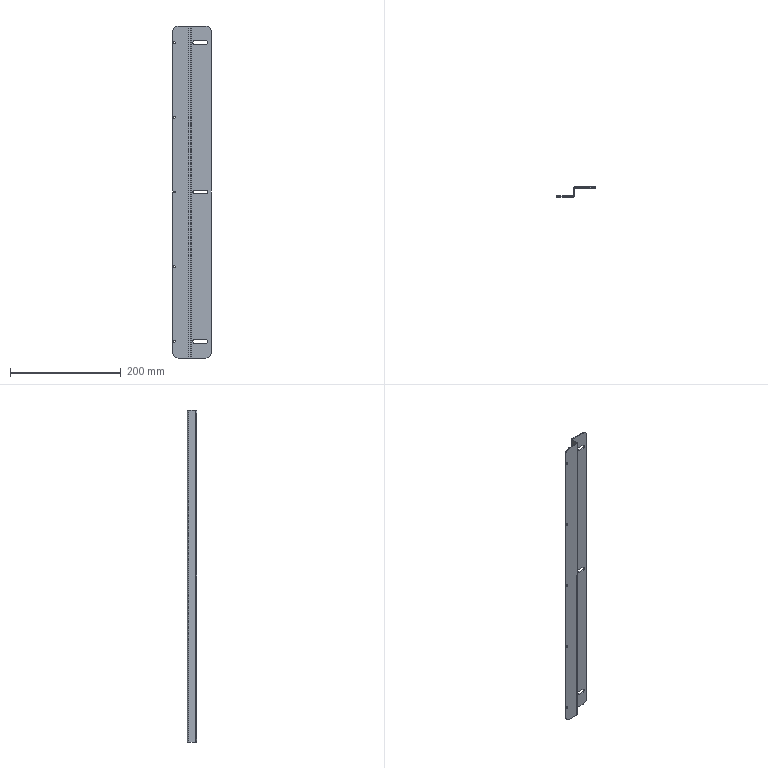Part | SolidWorks | features 3DProfileFeature 1, Fillet 1, FlatPattern 1, HoleWzd 1, ICE 1, SMBaseFlange 1, SheetMetal 1 | 1 solid | 51 faces | box 70 x 18 x 600 mm | volume 99365 mm3 | cylinder 27 | plane 24 | commonest cylinder face diameters 3.4 x10 6.6 x9 20 x4 3 x2 7 x2
STEP:
#1=CARTESIAN_POINT('',(-67.,-18.,-271.7));
#2=VERTEX_POINT('',#1);
#3=CARTESIAN_POINT('',(-67.,-18.,-268.3));
#4=VERTEX_POINT('',#3);
#5=CARTESIAN_POINT('',(-67.,-18.,-270.));
#6=DIRECTION('',(0.,1.,0.));
#7=DIRECTION('',(0.,0.,1.));
#8=AXIS2_PLACEMENT_3D('',#5,#6,#7);
#9=CIRCLE('',#8,1.7);
#10=EDGE_CURVE('',#2,#4,#9,.T.);
#11=ORIENTED_EDGE('',*,*,#10,.F.);
#12=CARTESIAN_POINT('',(-67.,-16.,-271.7));
#13=VERTEX_POINT('',#12);
#14=CARTESIAN_POINT('',(-67.,-16.,-271.7));
#15=DIRECTION('',(0.,1.,0.));
#16=VECTOR('',#15,1000.);
#17=LINE('',#14,#16);
#18=EDGE_CURVE('',#2,#13,#17,.T.);
#19=ORIENTED_EDGE('',*,*,#18,.T.);
#20=CARTESIAN_POINT('',(-67.,-16.,-268.3));
#21=VERTEX_POINT('',#20);
#22=CARTESIAN_POINT('',(-67.,-16.,-270.));
#23=DIRECTION('',(0.,1.,0.));
#24=DIRECTION('',(0.,0.,1.));
#25=AXIS2_PLACEMENT_3D('',#22,#23,#24);
#26=CIRCLE('',#25,1.7);
#27=EDGE_CURVE('',#13,#21,#26,.T.);
#28=ORIENTED_EDGE('',*,*,#27,.T.);
#29=CARTESIAN_POINT('',(-67.,-16.,-268.3));
#30=DIRECTION('',(0.,1.,0.));
#31=VECTOR('',#30,1000.);
#32=LINE('',#29,#31);
#33=EDGE_CURVE('',#4,#21,#32,.T.);
#34=ORIENTED_EDGE('',*,*,#33,.F.);
#35=EDGE_LOOP('',(#11,#19,#28,#34));
#36=FACE_OUTER_BOUND('',#35,.T.);
#37=CARTESIAN_POINT('',(-67.,-16.,-270.));
#38=DIRECTION('',(0.,1.,0.));
#39=DIRECTION('',(0.,0.,1.));
#40=AXIS2_PLACEMENT_3D('',#37,#38,#39);
#41=CYLINDRICAL_SURFACE('',#40,1.7);
#42=ADVANCED_FACE('',(#36),#41,.F.);
#43=CARTESIAN_POINT('',(-67.,-18.,-1.7));
#44=VERTEX_POINT('',#43);
#45=CARTESIAN_POINT('',(-67.,-18.,1.7));
#46=VERTEX_POINT('',#45);
#47=CARTESIAN_POINT('',(-67.,-18.,0.));
#48=DIRECTION('',(0.,1.,0.));
#49=DIRECTION('',(0.,0.,1.));
#50=AXIS2_PLACEMENT_3D('',#47,#48,#49);
#51=CIRCLE('',#50,1.7);
#52=EDGE_CURVE('',#44,#46,#51,.T.);
#53=ORIENTED_EDGE('',*,*,#52,.F.);
#54=CARTESIAN_POINT('',(-67.,-16.,-1.7));
#55=VERTEX_POINT('',#54);
#56=CARTESIAN_POINT('',(-67.,-16.,-1.7));
#57=DIRECTION('',(0.,1.,0.));
#58=VECTOR('',#57,1000.);
#59=LINE('',#56,#58);
#60=EDGE_CURVE('',#44,#55,#59,.T.);
#61=ORIENTED_EDGE('',*,*,#60,.T.);
#62=CARTESIAN_POINT('',(-67.,-16.,1.7));
#63=VERTEX_POINT('',#62);
#64=CARTESIAN_POINT('',(-67.,-16.,0.));
#65=DIRECTION('',(0.,1.,0.));
#66=DIRECTION('',(0.,0.,1.));
#67=AXIS2_PLACEMENT_3D('',#64,#65,#66);
#68=CIRCLE('',#67,1.7);
#69=EDGE_CURVE('',#55,#63,#68,.T.);
#70=ORIENTED_EDGE('',*,*,#69,.T.);
#71=CARTESIAN_POINT('',(-67.,-16.,1.7));
#72=DIRECTION('',(0.,1.,0.));
#73=VECTOR('',#72,1000.);
#74=LINE('',#71,#73);
#75=EDGE_CURVE('',#46,#63,#74,.T.);
#76=ORIENTED_EDGE('',*,*,#75,.F.);
#77=EDGE_LOOP('',(#53,#61,#70,#76));
#78=FACE_OUTER_BOUND('',#77,.T.);
#79=CARTESIAN_POINT('',(-67.,-16.,0.));
#80=DIRECTION('',(0.,1.,0.));
#81=DIRECTION('',(0.,0.,1.));
#82=AXIS2_PLACEMENT_3D('',#79,#80,#81);
#83=CYLINDRICAL_SURFACE('',#82,1.7);
#84=ADVANCED_FACE('',(#78),#83,.F.);
#85=CARTESIAN_POINT('',(-67.,-18.,268.3));
#86=VERTEX_POINT('',#85);
#87=CARTESIAN_POINT('',(-67.,-18.,271.7));
#88=VERTEX_POINT('',#87);
#89=CARTESIAN_POINT('',(-67.,-18.,270.));
#90=DIRECTION('',(0.,1.,0.));
#91=DIRECTION('',(0.,0.,1.));
#92=AXIS2_PLACEMENT_3D('',#89,#90,#91);
#93=CIRCLE('',#92,1.7);
#94=EDGE_CURVE('',#86,#88,#93,.T.);
#95=ORIENTED_EDGE('',*,*,#94,.F.);
#96=CARTESIAN_POINT('',(-67.,-16.,268.3));
#97=VERTEX_POINT('',#96);
#98=CARTESIAN_POINT('',(-67.,-16.,268.3));
#99=DIRECTION('',(0.,1.,0.));
#100=VECTOR('',#99,1000.);
#101=LINE('',#98,#100);
#102=EDGE_CURVE('',#86,#97,#101,.T.);
#103=ORIENTED_EDGE('',*,*,#102,.T.);
#104=CARTESIAN_POINT('',(-67.,-16.,271.7));
#105=VERTEX_POINT('',#104);
#106=CARTESIAN_POINT('',(-67.,-16.,270.));
#107=DIRECTION('',(0.,1.,0.));
#108=DIRECTION('',(0.,0.,1.));
#109=AXIS2_PLACEMENT_3D('',#106,#107,#108);
#110=CIRCLE('',#109,1.7);
#111=EDGE_CURVE('',#97,#105,#110,.T.);
#112=ORIENTED_EDGE('',*,*,#111,.T.);
#113=CARTESIAN_POINT('',(-67.,-16.,271.7));
#114=DIRECTION('',(0.,1.,0.));
#115=VECTOR('',#114,1000.);
#116=LINE('',#113,#115);
#117=EDGE_CURVE('',#88,#105,#116,.T.);
#118=ORIENTED_EDGE('',*,*,#117,.F.);
#119=EDGE_LOOP('',(#95,#103,#112,#118));
#120=FACE_OUTER_BOUND('',#119,.T.);
#121=CARTESIAN_POINT('',(-67.,-16.,270.));
#122=DIRECTION('',(0.,1.,0.));
#123=DIRECTION('',(0.,0.,1.));
#124=AXIS2_PLACEMENT_3D('',#121,#122,#123);
#125=CYLINDRICAL_SURFACE('',#124,1.7);
#126=ADVANCED_FACE('',(#120),#125,.F.);
#127=CARTESIAN_POINT('',(-67.,-18.,133.3));
#128=VERTEX_POINT('',#127);
#129=CARTESIAN_POINT('',(-67.,-18.,136.7));
#130=VERTEX_POINT('',#129);
#131=CARTESIAN_POINT('',(-67.,-18.,135.));
#132=DIRECTION('',(0.,1.,0.));
#133=DIRECTION('',(0.,0.,1.));
#134=AXIS2_PLACEMENT_3D('',#131,#132,#133);
#135=CIRCLE('',#134,1.7);
#136=EDGE_CURVE('',#128,#130,#135,.T.);
#137=ORIENTED_EDGE('',*,*,#136,.F.);
#138=CARTESIAN_POINT('',(-67.,-16.,133.3));
#139=VERTEX_POINT('',#138);
#140=CARTESIAN_POINT('',(-67.,-16.,133.3));
#141=DIRECTION('',(0.,1.,0.));
#142=VECTOR('',#141,1000.);
#143=LINE('',#140,#142);
#144=EDGE_CURVE('',#128,#139,#143,.T.);
#145=ORIENTED_EDGE('',*,*,#144,.T.);
#146=CARTESIAN_POINT('',(-67.,-16.,136.7));
#147=VERTEX_POINT('',#146);
#148=CARTESIAN_POINT('',(-67.,-16.,135.));
#149=DIRECTION('',(0.,1.,0.));
#150=DIRECTION('',(0.,0.,1.));
#151=AXIS2_PLACEMENT_3D('',#148,#149,#150);
#152=CIRCLE('',#151,1.7);
#153=EDGE_CURVE('',#139,#147,#152,.T.);
#154=ORIENTED_EDGE('',*,*,#153,.T.);
#155=CARTESIAN_POINT('',(-67.,-16.,136.7));
#156=DIRECTION('',(0.,1.,0.));
#157=VECTOR('',#156,1000.);
#158=LINE('',#155,#157);
#159=EDGE_CURVE('',#130,#147,#158,.T.);
#160=ORIENTED_EDGE('',*,*,#159,.F.);
#161=EDGE_LOOP('',(#137,#145,#154,#160));
#162=FACE_OUTER_BOUND('',#161,.T.);
#163=CARTESIAN_POINT('',(-67.,-16.,135.));
#164=DIRECTION('',(0.,1.,0.));
#165=DIRECTION('',(0.,0.,1.));
#166=AXIS2_PLACEMENT_3D('',#163,#164,#165);
#167=CYLINDRICAL_SURFACE('',#166,1.7);
#168=ADVANCED_FACE('',(#162),#167,.F.);
#169=CARTESIAN_POINT('',(-67.,-18.,-136.7));
#170=VERTEX_POINT('',#169);
#171=CARTESIAN_POINT('',(-67.,-18.,-133.3));
#172=VERTEX_POINT('',#171);
#173=CARTESIAN_POINT('',(-67.,-18.,-135.));
#174=DIRECTION('',(0.,1.,0.));
#175=DIRECTION('',(0.,0.,1.));
#176=AXIS2_PLACEMENT_3D('',#173,#174,#175);
#177=CIRCLE('',#176,1.7);
#178=EDGE_CURVE('',#170,#172,#177,.T.);
#179=ORIENTED_EDGE('',*,*,#178,.F.);
#180=CARTESIAN_POINT('',(-67.,-16.,-136.7));
#181=VERTEX_POINT('',#180);
#182=CARTESIAN_POINT('',(-67.,-16.,-136.7));
#183=DIRECTION('',(0.,1.,0.));
#184=VECTOR('',#183,1000.);
#185=LINE('',#182,#184);
#186=EDGE_CURVE('',#170,#181,#185,.T.);
#187=ORIENTED_EDGE('',*,*,#186,.T.);
#188=CARTESIAN_POINT('',(-67.,-16.,-133.3));
#189=VERTEX_POINT('',#188);
#190=CARTESIAN_POINT('',(-67.,-16.,-135.));
#191=DIRECTION('',(0.,1.,0.));
#192=DIRECTION('',(0.,0.,1.));
#193=AXIS2_PLACEMENT_3D('',#190,#191,#192);
#194=CIRCLE('',#193,1.7);
#195=EDGE_CURVE('',#181,#189,#194,.T.);
#196=ORIENTED_EDGE('',*,*,#195,.T.);
#197=CARTESIAN_POINT('',(-67.,-16.,-133.3));
#198=DIRECTION('',(0.,1.,0.));
#199=VECTOR('',#198,1000.);
#200=LINE('',#197,#199);
#201=EDGE_CURVE('',#172,#189,#200,.T.);
#202=ORIENTED_EDGE('',*,*,#201,.F.);
#203=EDGE_LOOP('',(#179,#187,#196,#202));
#204=FACE_OUTER_BOUND('',#203,.T.);
#205=CARTESIAN_POINT('',(-67.,-16.,-135.));
#206=DIRECTION('',(0.,1.,0.));
#207=DIRECTION('',(0.,0.,1.));
#208=AXIS2_PLACEMENT_3D('',#205,#206,#207);
#209=CYLINDRICAL_SURFACE('',#208,1.7);
#210=ADVANCED_FACE('',(#204),#209,.F.);
#211=CARTESIAN_POINT('',(-30.,-2.,-266.7));
#212=VERTEX_POINT('',#211);
#213=CARTESIAN_POINT('',(-33.3,-2.,-270.));
#214=VERTEX_POINT('',#213);
#215=CARTESIAN_POINT('',(-30.,-2.,-270.));
#216=DIRECTION('',(0.,-1.,0.));
#217=DIRECTION('',(1.,0.,0.));
#218=AXIS2_PLACEMENT_3D('',#215,#216,#217);
#219=CIRCLE('',#218,3.3);
#220=EDGE_CURVE('',#212,#214,#219,.T.);
#221=ORIENTED_EDGE('',*,*,#220,.T.);
#222=CARTESIAN_POINT('',(-33.3,0.,-270.));
#223=VERTEX_POINT('',#222);
#224=CARTESIAN_POINT('',(-33.3,-10.,-270.));
#225=DIRECTION('',(0.,1.,0.));
#226=VECTOR('',#225,1000.);
#227=LINE('',#224,#226);
#228=EDGE_CURVE('',#214,#223,#227,.T.);
#229=ORIENTED_EDGE('',*,*,#228,.T.);
#230=CARTESIAN_POINT('',(-30.,0.,-266.7));
#231=VERTEX_POINT('',#230);
#232=CARTESIAN_POINT('',(-30.,0.,-270.));
#233=DIRECTION('',(0.,1.,0.));
#234=DIRECTION('',(-1.,0.,0.));
#235=AXIS2_PLACEMENT_3D('',#232,#233,#234);
#236=CIRCLE('',#235,3.3);
#237=EDGE_CURVE('',#223,#231,#236,.T.);
#238=ORIENTED_EDGE('',*,*,#237,.T.);
#239=CARTESIAN_POINT('',(-30.,-10.,-266.7));
#240=DIRECTION('',(0.,1.,0.));
#241=VECTOR('',#240,1000.);
#242=LINE('',#239,#241);
#243=EDGE_CURVE('',#212,#231,#242,.T.);
#244=ORIENTED_EDGE('',*,*,#243,.F.);
#245=EDGE_LOOP('',(#221,#229,#238,#244));
#246=FACE_OUTER_BOUND('',#245,.T.);
#247=CARTESIAN_POINT('',(-30.,-10.,-270.));
#248=DIRECTION('',(0.,1.,0.));
#249=DIRECTION('',(-1.,0.,0.));
#250=AXIS2_PLACEMENT_3D('',#247,#248,#249);
#251=CYLINDRICAL_SURFACE('',#250,3.3);
#252=ADVANCED_FACE('',(#246),#251,.F.);
#253=CARTESIAN_POINT('',(-30.,-2.,3.3));
#254=VERTEX_POINT('',#253);
#255=CARTESIAN_POINT('',(-33.3,-2.,0.));
#256=VERTEX_POINT('',#255);
#257=CARTESIAN_POINT('',(-30.,-2.,0.));
#258=DIRECTION('',(0.,-1.,0.));
#259=DIRECTION('',(1.,0.,0.));
#260=AXIS2_PLACEMENT_3D('',#257,#258,#259);
#261=CIRCLE('',#260,3.3);
#262=EDGE_CURVE('',#254,#256,#261,.T.);
#263=ORIENTED_EDGE('',*,*,#262,.T.);
#264=CARTESIAN_POINT('',(-33.3,0.,0.));
#265=VERTEX_POINT('',#264);
#266=CARTESIAN_POINT('',(-33.3,-10.,0.));
#267=DIRECTION('',(0.,1.,0.));
#268=VECTOR('',#267,1000.);
#269=LINE('',#266,#268);
#270=EDGE_CURVE('',#256,#265,#269,.T.);
#271=ORIENTED_EDGE('',*,*,#270,.T.);
#272=CARTESIAN_POINT('',(-30.,0.,3.3));
#273=VERTEX_POINT('',#272);
#274=CARTESIAN_POINT('',(-30.,0.,0.));
#275=DIRECTION('',(0.,1.,0.));
#276=DIRECTION('',(-1.,0.,0.));
#277=AXIS2_PLACEMENT_3D('',#274,#275,#276);
#278=CIRCLE('',#277,3.3);
#279=EDGE_CURVE('',#265,#273,#278,.T.);
#280=ORIENTED_EDGE('',*,*,#279,.T.);
#281=CARTESIAN_POINT('',(-30.,-10.,3.3));
#282=DIRECTION('',(0.,1.,0.));
#283=VECTOR('',#282,1000.);
#284=LINE('',#281,#283);
#285=EDGE_CURVE('',#254,#273,#284,.T.);
#286=ORIENTED_EDGE('',*,*,#285,.F.);
#287=EDGE_LOOP('',(#263,#271,#280,#286));
#288=FACE_OUTER_BOUND('',#287,.T.);
#289=CARTESIAN_POINT('',(-30.,-10.,0.));
#290=DIRECTION('',(0.,1.,0.));
#291=DIRECTION('',(-1.,0.,0.));
#292=AXIS2_PLACEMENT_3D('',#289,#290,#291);
#293=CYLINDRICAL_SURFACE('',#292,3.3);
#294=ADVANCED_FACE('',(#288),#293,.F.);
#295=CARTESIAN_POINT('',(-30.,-2.,273.3));
#296=VERTEX_POINT('',#295);
#297=CARTESIAN_POINT('',(-33.3,-2.,270.));
#298=VERTEX_POINT('',#297);
#299=CARTESIAN_POINT('',(-30.,-2.,270.));
#300=DIRECTION('',(0.,-1.,0.));
#301=DIRECTION('',(1.,0.,0.));
#302=AXIS2_PLACEMENT_3D('',#299,#300,#301);
#303=CIRCLE('',#302,3.3);
#304=EDGE_CURVE('',#296,#298,#303,.T.);
#305=ORIENTED_EDGE('',*,*,#304,.T.);
#306=CARTESIAN_POINT('',(-33.3,0.,270.));
#307=VERTEX_POINT('',#306);
#308=CARTESIAN_POINT('',(-33.3,-10.,270.));
#309=DIRECTION('',(0.,1.,0.));
#310=VECTOR('',#309,1000.);
#311=LINE('',#308,#310);
#312=EDGE_CURVE('',#298,#307,#311,.T.);
#313=ORIENTED_EDGE('',*,*,#312,.T.);
#314=CARTESIAN_POINT('',(-30.,0.,273.3));
#315=VERTEX_POINT('',#314);
#316=CARTESIAN_POINT('',(-30.,0.,270.));
#317=DIRECTION('',(0.,1.,0.));
#318=DIRECTION('',(-1.,0.,0.));
#319=AXIS2_PLACEMENT_3D('',#316,#317,#318);
#320=CIRCLE('',#319,3.3);
#321=EDGE_CURVE('',#307,#315,#320,.T.);
#322=ORIENTED_EDGE('',*,*,#321,.T.);
#323=CARTESIAN_POINT('',(-30.,-10.,273.3));
#324=DIRECTION('',(0.,1.,0.));
#325=VECTOR('',#324,1000.);
#326=LINE('',#323,#325);
#327=EDGE_CURVE('',#296,#315,#326,.T.);
#328=ORIENTED_EDGE('',*,*,#327,.F.);
#329=EDGE_LOOP('',(#305,#313,#322,#328));
#330=FACE_OUTER_BOUND('',#329,.T.);
#331=CARTESIAN_POINT('',(-30.,-10.,270.));
#332=DIRECTION('',(0.,1.,0.));
#333=DIRECTION('',(-1.,0.,0.));
#334=AXIS2_PLACEMENT_3D('',#331,#332,#333);
#335=CYLINDRICAL_SURFACE('',#334,3.3);
#336=ADVANCED_FACE('',(#330),#335,.F.);
#337=CARTESIAN_POINT('',(-36.5,0.,300.));
#338=VERTEX_POINT('',#337);
#339=CARTESIAN_POINT('',(-36.5,-2.,300.));
#340=VERTEX_POINT('',#339);
#341=CARTESIAN_POINT('',(-36.5,0.,300.));
#342=DIRECTION('',(0.,-1.,0.));
#343=VECTOR('',#342,1000.);
#344=LINE('',#341,#343);
#345=EDGE_CURVE('',#338,#340,#344,.T.);
#346=ORIENTED_EDGE('',*,*,#345,.F.);
#347=CARTESIAN_POINT('',(-40.,-3.5,300.));
#348=VERTEX_POINT('',#347);
#349=CARTESIAN_POINT('',(-36.5,-3.5,300.));
#350=DIRECTION('',(0.,0.,1.));
#351=DIRECTION('',(-1.,0.,0.));
#352=AXIS2_PLACEMENT_3D('',#349,#350,#351);
#353=CIRCLE('',#352,3.5);
#354=EDGE_CURVE('',#338,#348,#353,.T.);
#355=ORIENTED_EDGE('',*,*,#354,.T.);
#356=CARTESIAN_POINT('',(-38.,-3.5,300.));
#357=VERTEX_POINT('',#356);
#358=CARTESIAN_POINT('',(-38.,-3.5,300.));
#359=DIRECTION('',(-1.,0.,0.));
#360=VECTOR('',#359,1000.);
#361=LINE('',#358,#360);
#362=EDGE_CURVE('',#357,#348,#361,.T.);
#363=ORIENTED_EDGE('',*,*,#362,.F.);
#364=CARTESIAN_POINT('',(-36.5,-3.5,300.));
#365=DIRECTION('',(0.,0.,1.));
#366=DIRECTION('',(1.,0.,0.));
#367=AXIS2_PLACEMENT_3D('',#364,#365,#366);
#368=CIRCLE('',#367,1.5);
#369=EDGE_CURVE('',#340,#357,#368,.T.);
#370=ORIENTED_EDGE('',*,*,#369,.F.);
#371=EDGE_LOOP('',(#346,#355,#363,#370));
#372=FACE_OUTER_BOUND('',#371,.T.);
#373=CARTESIAN_POINT('',(-36.5,0.,300.));
#374=DIRECTION('',(0.,0.,1.));
#375=DIRECTION('',(1.,0.,0.));
#376=AXIS2_PLACEMENT_3D('',#373,#374,#375);
#377=PLANE('',#376);
#378=ADVANCED_FACE('',(#372),#377,.T.);
#379=CARTESIAN_POINT('',(-10.,-2.,300.));
#380=VERTEX_POINT('',#379);
#381=CARTESIAN_POINT('',(0.,-2.,300.));
#382=DIRECTION('',(-1.,0.,0.));
#383=VECTOR('',#382,1000.);
#384=LINE('',#381,#383);
#385=EDGE_CURVE('',#380,#340,#384,.T.);
#386=ORIENTED_EDGE('',*,*,#385,.F.);
#387=CARTESIAN_POINT('',(-10.,0.,300.));
#388=VERTEX_POINT('',#387);
#389=CARTESIAN_POINT('',(-10.,-3.5,300.));
#390=DIRECTION('',(0.,1.,0.));
#391=VECTOR('',#390,1000.);
#392=LINE('',#389,#391);
#393=EDGE_CURVE('',#380,#388,#392,.T.);
#394=ORIENTED_EDGE('',*,*,#393,.T.);
#395=CARTESIAN_POINT('',(0.,0.,300.));
#396=DIRECTION('',(-1.,0.,0.));
#397=VECTOR('',#396,1000.);
#398=LINE('',#395,#397);
#399=EDGE_CURVE('',#388,#338,#398,.T.);
#400=ORIENTED_EDGE('',*,*,#399,.T.);
#401=ORIENTED_EDGE('',*,*,#345,.T.);
#402=EDGE_LOOP('',(#386,#394,#400,#401));
#403=FACE_OUTER_BOUND('',#402,.T.);
#404=CARTESIAN_POINT('',(-38.,-3.5,300.));
#405=DIRECTION('',(0.,0.,1.));
#406=DIRECTION('',(1.,0.,0.));
#407=AXIS2_PLACEMENT_3D('',#404,#405,#406);
#408=PLANE('',#407);
#409=ADVANCED_FACE('',(#403),#408,.T.);
#410=CARTESIAN_POINT('',(-40.,-3.5,-300.));
#411=VERTEX_POINT('',#410);
#412=CARTESIAN_POINT('',(-38.,-3.5,-300.));
#413=VERTEX_POINT('',#412);
#414=CARTESIAN_POINT('',(-40.,-3.5,-300.));
#415=DIRECTION('',(1.,0.,0.));
#416=VECTOR('',#415,1000.);
#417=LINE('',#414,#416);
#418=EDGE_CURVE('',#411,#413,#417,.T.);
#419=ORIENTED_EDGE('',*,*,#418,.F.);
#420=CARTESIAN_POINT('',(-36.5,0.,-300.));
#421=VERTEX_POINT('',#420);
#422=CARTESIAN_POINT('',(-36.5,-3.5,-300.));
#423=DIRECTION('',(0.,0.,1.));
#424=DIRECTION('',(-1.,0.,0.));
#425=AXIS2_PLACEMENT_3D('',#422,#423,#424);
#426=CIRCLE('',#425,3.5);
#427=EDGE_CURVE('',#421,#411,#426,.T.);
#428=ORIENTED_EDGE('',*,*,#427,.F.);
#429=CARTESIAN_POINT('',(-36.5,-2.,-300.));
#430=VERTEX_POINT('',#429);
#431=CARTESIAN_POINT('',(-36.5,-2.,-300.));
#432=DIRECTION('',(0.,1.,0.));
#433=VECTOR('',#432,1000.);
#434=LINE('',#431,#433);
#435=EDGE_CURVE('',#430,#421,#434,.T.);
#436=ORIENTED_EDGE('',*,*,#435,.F.);
#437=CARTESIAN_POINT('',(-36.5,-3.5,-300.));
#438=DIRECTION('',(0.,0.,1.));
#439=DIRECTION('',(1.,0.,0.));
#440=AXIS2_PLACEMENT_3D('',#437,#438,#439);
#441=CIRCLE('',#440,1.5);
#442=EDGE_CURVE('',#430,#413,#441,.T.);
#443=ORIENTED_EDGE('',*,*,#442,.T.);
#444=EDGE_LOOP('',(#419,#428,#436,#443));
#445=FACE_OUTER_BOUND('',#444,.T.);
#446=CARTESIAN_POINT('',(-40.,-3.5,-300.));
#447=DIRECTION('',(0.,0.,-1.));
#448=DIRECTION('',(-1.,0.,0.));
#449=AXIS2_PLACEMENT_3D('',#446,#447,#448);
#450=PLANE('',#449);
#451=ADVANCED_FACE('',(#445),#450,.T.);
#452=CARTESIAN_POINT('',(-40.,-14.5,-300.));
#453=VERTEX_POINT('',#452);
#454=CARTESIAN_POINT('',(-40.,0.,-300.));
#455=DIRECTION('',(0.,-1.,0.));
#456=VECTOR('',#455,1000.);
#457=LINE('',#454,#456);
#458=EDGE_CURVE('',#411,#453,#457,.T.);
#459=ORIENTED_EDGE('',*,*,#458,.F.);
#460=ORIENTED_EDGE('',*,*,#418,.T.);
#461=CARTESIAN_POINT('',(-38.,-14.5,-300.));
#462=VERTEX_POINT('',#461);
#463=CARTESIAN_POINT('',(-38.,0.,-300.));
#464=DIRECTION('',(0.,-1.,0.));
#465=VECTOR('',#464,1000.);
#466=LINE('',#463,#465);
#467=EDGE_CURVE('',#413,#462,#466,.T.);
#468=ORIENTED_EDGE('',*,*,#467,.T.);
#469=CARTESIAN_POINT('',(-38.,-14.5,-300.));
#470=DIRECTION('',(-1.,0.,0.));
#471=VECTOR('',#470,1000.);
#472=LINE('',#469,#471);
#473=EDGE_CURVE('',#462,#453,#472,.T.);
#474=ORIENTED_EDGE('',*,*,#473,.T.);
#475=EDGE_LOOP('',(#459,#460,#468,#474));
#476=FACE_OUTER_BOUND('',#475,.T.);
#477=CARTESIAN_POINT('',(-36.5,-2.,-300.));
#478=DIRECTION('',(0.,0.,-1.));
#479=DIRECTION('',(-1.,0.,0.));
#480=AXIS2_PLACEMENT_3D('',#477,#478,#479);
#481=PLANE('',#480);
#482=ADVANCED_FACE('',(#476),#481,.T.);
#483=CARTESIAN_POINT('',(-40.,-14.5,300.));
#484=VERTEX_POINT('',#483);
#485=CARTESIAN_POINT('',(-38.,-14.5,300.));
#486=VERTEX_POINT('',#485);
#487=CARTESIAN_POINT('',(-40.,-14.5,300.));
#488=DIRECTION('',(1.,0.,0.));
#489=VECTOR('',#488,1000.);
#490=LINE('',#487,#489);
#491=EDGE_CURVE('',#484,#486,#490,.T.);
#492=ORIENTED_EDGE('',*,*,#491,.F.);
#493=CARTESIAN_POINT('',(-41.5,-16.,300.));
#494=VERTEX_POINT('',#493);
#495=CARTESIAN_POINT('',(-41.5,-14.5,300.));
#496=DIRECTION('',(0.,0.,-1.));
#497=DIRECTION('',(1.,0.,0.));
#498=AXIS2_PLACEMENT_3D('',#495,#496,#497);
#499=CIRCLE('',#498,1.5);
#500=EDGE_CURVE('',#484,#494,#499,.T.);
#501=ORIENTED_EDGE('',*,*,#500,.T.);
#502=CARTESIAN_POINT('',(-41.5,-18.,300.));
#503=VERTEX_POINT('',#502);
#504=CARTESIAN_POINT('',(-41.5,-18.,300.));
#505=DIRECTION('',(0.,1.,0.));
#506=VECTOR('',#505,1000.);
#507=LINE('',#504,#506);
#508=EDGE_CURVE('',#503,#494,#507,.T.);
#509=ORIENTED_EDGE('',*,*,#508,.F.);
#510=CARTESIAN_POINT('',(-41.5,-14.5,300.));
#511=DIRECTION('',(0.,0.,-1.));
#512=DIRECTION('',(1.,0.,0.));
#513=AXIS2_PLACEMENT_3D('',#510,#511,#512);
#514=CIRCLE('',#513,3.5);
#515=EDGE_CURVE('',#486,#503,#514,.T.);
#516=ORIENTED_EDGE('',*,*,#515,.F.);
#517=EDGE_LOOP('',(#492,#501,#509,#516));
#518=FACE_OUTER_BOUND('',#517,.T.);
#519=CARTESIAN_POINT('',(-40.,-14.5,300.));
#520=DIRECTION('',(0.,0.,1.));
#521=DIRECTION('',(1.,0.,0.));
#522=AXIS2_PLACEMENT_3D('',#519,#520,#521);
#523=PLANE('',#522);
#524=ADVANCED_FACE('',(#518),#523,.T.);
#525=CARTESIAN_POINT('',(-40.,0.,300.));
#526=DIRECTION('',(0.,-1.,0.));
#527=VECTOR('',#526,1000.);
#528=LINE('',#525,#527);
#529=EDGE_CURVE('',#348,#484,#528,.T.);
#530=ORIENTED_EDGE('',*,*,#529,.T.);
#531=ORIENTED_EDGE('',*,*,#491,.T.);
#532=CARTESIAN_POINT('',(-38.,0.,300.));
#533=DIRECTION('',(0.,-1.,0.));
#534=VECTOR('',#533,1000.);
#535=LINE('',#532,#534);
#536=EDGE_CURVE('',#357,#486,#535,.T.);
#537=ORIENTED_EDGE('',*,*,#536,.F.);
#538=ORIENTED_EDGE('',*,*,#362,.T.);
#539=EDGE_LOOP('',(#530,#531,#537,#538));
#540=FACE_OUTER_BOUND('',#539,.T.);
#541=CARTESIAN_POINT('',(-41.5,-18.,300.));
#542=DIRECTION('',(0.,0.,1.));
#543=DIRECTION('',(1.,0.,0.));
#544=AXIS2_PLACEMENT_3D('',#541,#542,#543);
#545=PLANE('',#544);
#546=ADVANCED_FACE('',(#540),#545,.T.);
#547=CARTESIAN_POINT('',(-41.5,-16.,-300.));
#548=VERTEX_POINT('',#547);
#549=CARTESIAN_POINT('',(-41.5,-18.,-300.));
#550=VERTEX_POINT('',#549);
#551=CARTESIAN_POINT('',(-41.5,-16.,-300.));
#552=DIRECTION('',(0.,-1.,0.));
#553=VECTOR('',#552,1000.);
#554=LINE('',#551,#553);
#555=EDGE_CURVE('',#548,#550,#554,.T.);
#556=ORIENTED_EDGE('',*,*,#555,.F.);
#557=CARTESIAN_POINT('',(-41.5,-14.5,-300.));
#558=DIRECTION('',(0.,0.,-1.));
#559=DIRECTION('',(1.,0.,0.));
#560=AXIS2_PLACEMENT_3D('',#557,#558,#559);
#561=CIRCLE('',#560,1.5);
#562=EDGE_CURVE('',#453,#548,#561,.T.);
#563=ORIENTED_EDGE('',*,*,#562,.F.);
#564=ORIENTED_EDGE('',*,*,#473,.F.);
#565=CARTESIAN_POINT('',(-41.5,-14.5,-300.));
#566=DIRECTION('',(0.,0.,-1.));
#567=DIRECTION('',(1.,0.,0.));
#568=AXIS2_PLACEMENT_3D('',#565,#566,#567);
#569=CIRCLE('',#568,3.5);
#570=EDGE_CURVE('',#462,#550,#569,.T.);
#571=ORIENTED_EDGE('',*,*,#570,.T.);
#572=EDGE_LOOP('',(#556,#563,#564,#571));
#573=FACE_OUTER_BOUND('',#572,.T.);
#574=CARTESIAN_POINT('',(-41.5,-16.,-300.));
#575=DIRECTION('',(0.,0.,-1.));
#576=DIRECTION('',(-1.,0.,0.));
#577=AXIS2_PLACEMENT_3D('',#574,#575,#576);
#578=PLANE('',#577);
#579=ADVANCED_FACE('',(#573),#578,.T.);
#580=CARTESIAN_POINT('',(-60.,-18.,-300.));
#581=VERTEX_POINT('',#580);
#582=CARTESIAN_POINT('',(-40.,-18.,-300.));
#583=DIRECTION('',(-1.,0.,0.));
#584=VECTOR('',#583,1000.);
#585=LINE('',#582,#584);
#586=EDGE_CURVE('',#550,#581,#585,.T.);
#587=ORIENTED_EDGE('',*,*,#586,.T.);
#588=CARTESIAN_POINT('',(-60.,-16.,-300.));
#589=VERTEX_POINT('',#588);
#590=CARTESIAN_POINT('',(-60.,-14.5,-300.));
#591=DIRECTION('',(0.,1.,0.));
#592=VECTOR('',#591,1000.);
#593=LINE('',#590,#592);
#594=EDGE_CURVE('',#581,#589,#593,.T.);
#595=ORIENTED_EDGE('',*,*,#594,.T.);
#596=CARTESIAN_POINT('',(-40.,-16.,-300.));
#597=DIRECTION('',(-1.,0.,0.));
#598=VECTOR('',#597,1000.);
#599=LINE('',#596,#598);
#600=EDGE_CURVE('',#548,#589,#599,.T.);
#601=ORIENTED_EDGE('',*,*,#600,.F.);
#602=ORIENTED_EDGE('',*,*,#555,.T.);
#603=EDGE_LOOP('',(#587,#595,#601,#602));
#604=FACE_OUTER_BOUND('',#603,.T.);
#605=CARTESIAN_POINT('',(-38.,-14.5,-300.));
#606=DIRECTION('',(0.,0.,-1.));
#607=DIRECTION('',(-1.,0.,0.));
#608=AXIS2_PLACEMENT_3D('',#605,#606,#607);
#609=PLANE('',#608);
#610=ADVANCED_FACE('',(#604),#609,.T.);
#611=CARTESIAN_POINT('',(-67.,-16.,-270.));
#612=DIRECTION('',(0.,1.,0.));
#613=DIRECTION('',(0.,0.,1.));
#614=AXIS2_PLACEMENT_3D('',#611,#612,#613);
#615=CIRCLE('',#614,1.7);
#616=EDGE_CURVE('',#21,#13,#615,.T.);
#617=ORIENTED_EDGE('',*,*,#616,.F.);
#618=ORIENTED_EDGE('',*,*,#27,.F.);
#619=EDGE_LOOP('',(#617,#618));
#620=FACE_BOUND('',#619,.T.);
#621=CARTESIAN_POINT('',(-67.,-16.,0.));
#622=DIRECTION('',(0.,1.,0.));
#623=DIRECTION('',(0.,0.,1.));
#624=AXIS2_PLACEMENT_3D('',#621,#622,#623);
#625=CIRCLE('',#624,1.7);
#626=EDGE_CURVE('',#63,#55,#625,.T.);
#627=ORIENTED_EDGE('',*,*,#626,.F.);
#628=ORIENTED_EDGE('',*,*,#69,.F.);
#629=EDGE_LOOP('',(#627,#628));
#630=FACE_BOUND('',#629,.T.);
#631=CARTESIAN_POINT('',(-67.,-16.,270.));
#632=DIRECTION('',(0.,1.,0.));
#633=DIRECTION('',(0.,0.,1.));
#634=AXIS2_PLACEMENT_3D('',#631,#632,#633);
#635=CIRCLE('',#634,1.7);
#636=EDGE_CURVE('',#105,#97,#635,.T.);
#637=ORIENTED_EDGE('',*,*,#636,.F.);
#638=ORIENTED_EDGE('',*,*,#111,.F.);
#639=EDGE_LOOP('',(#637,#638));
#640=FACE_BOUND('',#639,.T.);
#641=CARTESIAN_POINT('',(-67.,-16.,135.));
#642=DIRECTION('',(0.,1.,0.));
#643=DIRECTION('',(0.,0.,1.));
#644=AXIS2_PLACEMENT_3D('',#641,#642,#643);
#645=CIRCLE('',#644,1.7);
#646=EDGE_CURVE('',#147,#139,#645,.T.);
#647=ORIENTED_EDGE('',*,*,#646,.F.);
#648=ORIENTED_EDGE('',*,*,#153,.F.);
#649=EDGE_LOOP('',(#647,#648));
#650=FACE_BOUND('',#649,.T.);
#651=CARTESIAN_POINT('',(-67.,-16.,-135.));
#652=DIRECTION('',(0.,1.,0.));
#653=DIRECTION('',(0.,0.,1.));
#654=AXIS2_PLACEMENT_3D('',#651,#652,#653);
#655=CIRCLE('',#654,1.7);
#656=EDGE_CURVE('',#189,#181,#655,.T.);
#657=ORIENTED_EDGE('',*,*,#656,.F.);
#658=ORIENTED_EDGE('',*,*,#195,.F.);
#659=EDGE_LOOP('',(#657,#658));
#660=FACE_BOUND('',#659,.T.);
#661=ORIENTED_EDGE('',*,*,#600,.T.);
#662=CARTESIAN_POINT('',(-70.,-16.,-290.));
#663=VERTEX_POINT('',#662);
#664=CARTESIAN_POINT('',(-60.,-16.,-290.));
#665=DIRECTION('',(0.,1.,0.));
#666=DIRECTION('',(1.,0.,0.));
#667=AXIS2_PLACEMENT_3D('',#664,#665,#666);
#668=CIRCLE('',#667,10.);
#669=EDGE_CURVE('',#589,#663,#668,.T.);
#670=ORIENTED_EDGE('',*,*,#669,.T.);
#671=CARTESIAN_POINT('',(-70.,-16.,290.));
#672=VERTEX_POINT('',#671);
#673=CARTESIAN_POINT('',(-70.,-16.,300.));
#674=DIRECTION('',(0.,0.,-1.));
#675=VECTOR('',#674,1000.);
#676=LINE('',#673,#675);
#677=EDGE_CURVE('',#672,#663,#676,.T.);
#678=ORIENTED_EDGE('',*,*,#677,.F.);
#679=CARTESIAN_POINT('',(-60.,-16.,300.));
#680=VERTEX_POINT('',#679);
#681=CARTESIAN_POINT('',(-60.,-16.,290.));
#682=DIRECTION('',(0.,1.,0.));
#683=DIRECTION('',(1.,0.,0.));
#684=AXIS2_PLACEMENT_3D('',#681,#682,#683);
#685=CIRCLE('',#684,10.);
#686=EDGE_CURVE('',#672,#680,#685,.T.);
#687=ORIENTED_EDGE('',*,*,#686,.T.);
#688=CARTESIAN_POINT('',(-40.,-16.,300.));
#689=DIRECTION('',(-1.,0.,0.));
#690=VECTOR('',#689,1000.);
#691=LINE('',#688,#690);
#692=EDGE_CURVE('',#494,#680,#691,.T.);
#693=ORIENTED_EDGE('',*,*,#692,.F.);
#694=CARTESIAN_POINT('',(-41.5,-16.,300.));
#695=DIRECTION('',(0.,0.,-1.));
#696=VECTOR('',#695,1000.);
#697=LINE('',#694,#696);
#698=EDGE_CURVE('',#494,#548,#697,.T.);
#699=ORIENTED_EDGE('',*,*,#698,.T.);
#700=EDGE_LOOP('',(#661,#670,#678,#687,#693,#699));
#701=FACE_OUTER_BOUND('',#700,.T.);
#702=CARTESIAN_POINT('',(-40.,-16.,300.));
#703=DIRECTION('',(0.,-1.,0.));
#704=DIRECTION('',(1.,0.,0.));
#705=AXIS2_PLACEMENT_3D('',#702,#703,#704);
#706=PLANE('',#705);
#707=ADVANCED_FACE('',(#620,#630,#640,#650,#660,#701),#706,.F.);
#708=ORIENTED_EDGE('',*,*,#677,.T.);
#709=CARTESIAN_POINT('',(-70.,-18.,-290.));
#710=VERTEX_POINT('',#709);
#711=CARTESIAN_POINT('',(-70.,-18.,-290.));
#712=DIRECTION('',(0.,-1.,0.));
#713=VECTOR('',#712,1000.);
#714=LINE('',#711,#713);
#715=EDGE_CURVE('',#663,#710,#714,.T.);
#716=ORIENTED_EDGE('',*,*,#715,.T.);
#717=CARTESIAN_POINT('',(-70.,-18.,290.));
#718=VERTEX_POINT('',#717);
#719=CARTESIAN_POINT('',(-70.,-18.,300.));
#720=DIRECTION('',(0.,0.,-1.));
#721=VECTOR('',#720,1000.);
#722=LINE('',#719,#721);
#723=EDGE_CURVE('',#718,#710,#722,.T.);
#724=ORIENTED_EDGE('',*,*,#723,.F.);
#725=CARTESIAN_POINT('',(-70.,-18.,290.));
#726=DIRECTION('',(0.,1.,0.));
#727=VECTOR('',#726,1000.);
#728=LINE('',#725,#727);
#729=EDGE_CURVE('',#718,#672,#728,.T.);
#730=ORIENTED_EDGE('',*,*,#729,.T.);
#731=EDGE_LOOP('',(#708,#716,#724,#730));
#732=FACE_OUTER_BOUND('',#731,.T.);
#733=CARTESIAN_POINT('',(-70.,-18.,300.));
#734=DIRECTION('',(-1.,0.,0.));
#735=DIRECTION('',(0.,0.,1.));
#736=AXIS2_PLACEMENT_3D('',#733,#734,#735);
#737=PLANE('',#736);
#738=ADVANCED_FACE('',(#732),#737,.T.);
#739=CARTESIAN_POINT('',(-67.,-18.,-270.));
#740=DIRECTION('',(0.,1.,0.));
#741=DIRECTION('',(0.,0.,1.));
#742=AXIS2_PLACEMENT_3D('',#739,#740,#741);
#743=CIRCLE('',#742,1.7);
#744=EDGE_CURVE('',#4,#2,#743,.T.);
#745=ORIENTED_EDGE('',*,*,#744,.T.);
#746=ORIENTED_EDGE('',*,*,#10,.T.);
#747=EDGE_LOOP('',(#745,#746));
#748=FACE_BOUND('',#747,.T.);
#749=CARTESIAN_POINT('',(-67.,-18.,0.));
#750=DIRECTION('',(0.,1.,0.));
#751=DIRECTION('',(0.,0.,1.));
#752=AXIS2_PLACEMENT_3D('',#749,#750,#751);
#753=CIRCLE('',#752,1.7);
#754=EDGE_CURVE('',#46,#44,#753,.T.);
#755=ORIENTED_EDGE('',*,*,#754,.T.);
#756=ORIENTED_EDGE('',*,*,#52,.T.);
#757=EDGE_LOOP('',(#755,#756));
#758=FACE_BOUND('',#757,.T.);
#759=CARTESIAN_POINT('',(-67.,-18.,270.));
#760=DIRECTION('',(0.,1.,0.));
#761=DIRECTION('',(0.,0.,1.));
#762=AXIS2_PLACEMENT_3D('',#759,#760,#761);
#763=CIRCLE('',#762,1.7);
#764=EDGE_CURVE('',#88,#86,#763,.T.);
#765=ORIENTED_EDGE('',*,*,#764,.T.);
#766=ORIENTED_EDGE('',*,*,#94,.T.);
#767=EDGE_LOOP('',(#765,#766));
#768=FACE_BOUND('',#767,.T.);
#769=CARTESIAN_POINT('',(-67.,-18.,135.));
#770=DIRECTION('',(0.,1.,0.));
#771=DIRECTION('',(0.,0.,1.));
#772=AXIS2_PLACEMENT_3D('',#769,#770,#771);
#773=CIRCLE('',#772,1.7);
#774=EDGE_CURVE('',#130,#128,#773,.T.);
#775=ORIENTED_EDGE('',*,*,#774,.T.);
#776=ORIENTED_EDGE('',*,*,#136,.T.);
#777=EDGE_LOOP('',(#775,#776));
#778=FACE_BOUND('',#777,.T.);
#779=CARTESIAN_POINT('',(-67.,-18.,-135.));
#780=DIRECTION('',(0.,1.,0.));
#781=DIRECTION('',(0.,0.,1.));
#782=AXIS2_PLACEMENT_3D('',#779,#780,#781);
#783=CIRCLE('',#782,1.7);
#784=EDGE_CURVE('',#172,#170,#783,.T.);
#785=ORIENTED_EDGE('',*,*,#784,.T.);
#786=ORIENTED_EDGE('',*,*,#178,.T.);
#787=EDGE_LOOP('',(#785,#786));
#788=FACE_BOUND('',#787,.T.);
#789=ORIENTED_EDGE('',*,*,#723,.T.);
#790=CARTESIAN_POINT('',(-60.,-18.,-290.));
#791=DIRECTION('',(0.,-1.,0.));
#792=DIRECTION('',(1.,0.,0.));
#793=AXIS2_PLACEMENT_3D('',#790,#791,#792);
#794=CIRCLE('',#793,10.);
#795=EDGE_CURVE('',#710,#581,#794,.T.);
#796=ORIENTED_EDGE('',*,*,#795,.T.);
#797=ORIENTED_EDGE('',*,*,#586,.F.);
#798=CARTESIAN_POINT('',(-41.5,-18.,300.));
#799=DIRECTION('',(0.,0.,-1.));
#800=VECTOR('',#799,1000.);
#801=LINE('',#798,#800);
#802=EDGE_CURVE('',#503,#550,#801,.T.);
#803=ORIENTED_EDGE('',*,*,#802,.F.);
#804=CARTESIAN_POINT('',(-60.,-18.,300.));
#805=VERTEX_POINT('',#804);
#806=CARTESIAN_POINT('',(-40.,-18.,300.));
#807=DIRECTION('',(-1.,0.,0.));
#808=VECTOR('',#807,1000.);
#809=LINE('',#806,#808);
#810=EDGE_CURVE('',#503,#805,#809,.T.);
#811=ORIENTED_EDGE('',*,*,#810,.T.);
#812=CARTESIAN_POINT('',(-60.,-18.,290.));
#813=DIRECTION('',(0.,-1.,0.));
#814=DIRECTION('',(1.,0.,0.));
#815=AXIS2_PLACEMENT_3D('',#812,#813,#814);
#816=CIRCLE('',#815,10.);
#817=EDGE_CURVE('',#805,#718,#816,.T.);
#818=ORIENTED_EDGE('',*,*,#817,.T.);
#819=EDGE_LOOP('',(#789,#796,#797,#803,#811,#818));
#820=FACE_OUTER_BOUND('',#819,.T.);
#821=CARTESIAN_POINT('',(-40.,-18.,300.));
#822=DIRECTION('',(0.,-1.,0.));
#823=DIRECTION('',(1.,0.,0.));
#824=AXIS2_PLACEMENT_3D('',#821,#822,#823);
#825=PLANE('',#824);
#826=ADVANCED_FACE('',(#748,#758,#768,#778,#788,#820),#825,.T.);
#827=ORIENTED_EDGE('',*,*,#570,.F.);
#828=CARTESIAN_POINT('',(-38.,-14.5,300.));
#829=DIRECTION('',(0.,0.,-1.));
#830=VECTOR('',#829,1000.);
#831=LINE('',#828,#830);
#832=EDGE_CURVE('',#486,#462,#831,.T.);
#833=ORIENTED_EDGE('',*,*,#832,.F.);
#834=ORIENTED_EDGE('',*,*,#515,.T.);
#835=ORIENTED_EDGE('',*,*,#802,.T.);
#836=EDGE_LOOP('',(#827,#833,#834,#835));
#837=FACE_OUTER_BOUND('',#836,.T.);
#838=CARTESIAN_POINT('',(-41.5,-14.5,300.));
#839=DIRECTION('',(0.,0.,-1.));
#840=DIRECTION('',(-1.,0.,0.));
#841=AXIS2_PLACEMENT_3D('',#838,#839,#840);
#842=CYLINDRICAL_SURFACE('',#841,3.5);
#843=ADVANCED_FACE('',(#837),#842,.T.);
#844=ORIENTED_EDGE('',*,*,#467,.F.);
#845=CARTESIAN_POINT('',(-38.,-3.5,300.));
#846=DIRECTION('',(0.,0.,-1.));
#847=VECTOR('',#846,1000.);
#848=LINE('',#845,#847);
#849=EDGE_CURVE('',#357,#413,#848,.T.);
#850=ORIENTED_EDGE('',*,*,#849,.F.);
#851=ORIENTED_EDGE('',*,*,#536,.T.);
#852=ORIENTED_EDGE('',*,*,#832,.T.);
#853=EDGE_LOOP('',(#844,#850,#851,#852));
#854=FACE_OUTER_BOUND('',#853,.T.);
#855=CARTESIAN_POINT('',(-38.,0.,300.));
#856=DIRECTION('',(1.,0.,0.));
#857=DIRECTION('',(0.,0.,-1.));
#858=AXIS2_PLACEMENT_3D('',#855,#856,#857);
#859=PLANE('',#858);
#860=ADVANCED_FACE('',(#854),#859,.T.);
#861=ORIENTED_EDGE('',*,*,#442,.F.);
#862=CARTESIAN_POINT('',(-36.5,-2.,300.));
#863=DIRECTION('',(0.,0.,-1.));
#864=VECTOR('',#863,1000.);
#865=LINE('',#862,#864);
#866=EDGE_CURVE('',#340,#430,#865,.T.);
#867=ORIENTED_EDGE('',*,*,#866,.F.);
#868=ORIENTED_EDGE('',*,*,#369,.T.);
#869=ORIENTED_EDGE('',*,*,#849,.T.);
#870=EDGE_LOOP('',(#861,#867,#868,#869));
#871=FACE_OUTER_BOUND('',#870,.T.);
#872=CARTESIAN_POINT('',(-36.5,-3.5,300.));
#873=DIRECTION('',(0.,0.,-1.));
#874=DIRECTION('',(-1.,0.,0.));
#875=AXIS2_PLACEMENT_3D('',#872,#873,#874);
#876=CYLINDRICAL_SURFACE('',#875,1.5);
#877=ADVANCED_FACE('',(#871),#876,.F.);
#878=ORIENTED_EDGE('',*,*,#220,.F.);
#879=CARTESIAN_POINT('',(-10.,-2.,-266.7));
#880=VERTEX_POINT('',#879);
#881=CARTESIAN_POINT('',(0.,-2.,-266.7));
#882=DIRECTION('',(-1.,0.,0.));
#883=VECTOR('',#882,1000.);
#884=LINE('',#881,#883);
#885=EDGE_CURVE('',#880,#212,#884,.T.);
#886=ORIENTED_EDGE('',*,*,#885,.F.);
#887=CARTESIAN_POINT('',(-10.,-2.,-273.3));
#888=VERTEX_POINT('',#887);
#889=CARTESIAN_POINT('',(-10.,-2.,-270.));
#890=DIRECTION('',(0.,-1.,0.));
#891=DIRECTION('',(1.,0.,0.));
#892=AXIS2_PLACEMENT_3D('',#889,#890,#891);
#893=CIRCLE('',#892,3.3);
#894=EDGE_CURVE('',#888,#880,#893,.T.);
#895=ORIENTED_EDGE('',*,*,#894,.F.);
#896=CARTESIAN_POINT('',(-30.,-2.,-273.3));
#897=VERTEX_POINT('',#896);
#898=CARTESIAN_POINT('',(0.,-2.,-273.3));
#899=DIRECTION('',(1.,0.,0.));
#900=VECTOR('',#899,1000.);
#901=LINE('',#898,#900);
#902=EDGE_CURVE('',#897,#888,#901,.T.);
#903=ORIENTED_EDGE('',*,*,#902,.F.);
#904=CARTESIAN_POINT('',(-30.,-2.,-270.));
#905=DIRECTION('',(0.,-1.,0.));
#906=DIRECTION('',(1.,0.,0.));
#907=AXIS2_PLACEMENT_3D('',#904,#905,#906);
#908=CIRCLE('',#907,3.3);
#909=EDGE_CURVE('',#214,#897,#908,.T.);
#910=ORIENTED_EDGE('',*,*,#909,.F.);
#911=EDGE_LOOP('',(#878,#886,#895,#903,#910));
#912=FACE_BOUND('',#911,.T.);
#913=ORIENTED_EDGE('',*,*,#262,.F.);
#914=CARTESIAN_POINT('',(-10.,-2.,3.3));
#915=VERTEX_POINT('',#914);
#916=CARTESIAN_POINT('',(0.,-2.,3.3));
#917=DIRECTION('',(-1.,0.,0.));
#918=VECTOR('',#917,1000.);
#919=LINE('',#916,#918);
#920=EDGE_CURVE('',#915,#254,#919,.T.);
#921=ORIENTED_EDGE('',*,*,#920,.F.);
#922=CARTESIAN_POINT('',(-10.,-2.,-3.3));
#923=VERTEX_POINT('',#922);
#924=CARTESIAN_POINT('',(-10.,-2.,0.));
#925=DIRECTION('',(0.,-1.,0.));
#926=DIRECTION('',(1.,0.,0.));
#927=AXIS2_PLACEMENT_3D('',#924,#925,#926);
#928=CIRCLE('',#927,3.3);
#929=EDGE_CURVE('',#923,#915,#928,.T.);
#930=ORIENTED_EDGE('',*,*,#929,.F.);
#931=CARTESIAN_POINT('',(-30.,-2.,-3.3));
#932=VERTEX_POINT('',#931);
#933=CARTESIAN_POINT('',(0.,-2.,-3.3));
#934=DIRECTION('',(1.,0.,0.));
#935=VECTOR('',#934,1000.);
#936=LINE('',#933,#935);
#937=EDGE_CURVE('',#932,#923,#936,.T.);
#938=ORIENTED_EDGE('',*,*,#937,.F.);
#939=CARTESIAN_POINT('',(-30.,-2.,0.));
#940=DIRECTION('',(0.,-1.,0.));
#941=DIRECTION('',(1.,0.,0.));
#942=AXIS2_PLACEMENT_3D('',#939,#940,#941);
#943=CIRCLE('',#942,3.3);
#944=EDGE_CURVE('',#256,#932,#943,.T.);
#945=ORIENTED_EDGE('',*,*,#944,.F.);
#946=EDGE_LOOP('',(#913,#921,#930,#938,#945));
#947=FACE_BOUND('',#946,.T.);
#948=ORIENTED_EDGE('',*,*,#304,.F.);
#949=CARTESIAN_POINT('',(-10.,-2.,273.3));
#950=VERTEX_POINT('',#949);
#951=CARTESIAN_POINT('',(0.,-2.,273.3));
#952=DIRECTION('',(-1.,0.,0.));
#953=VECTOR('',#952,1000.);
#954=LINE('',#951,#953);
#955=EDGE_CURVE('',#950,#296,#954,.T.);
#956=ORIENTED_EDGE('',*,*,#955,.F.);
#957=CARTESIAN_POINT('',(-10.,-2.,266.7));
#958=VERTEX_POINT('',#957);
#959=CARTESIAN_POINT('',(-10.,-2.,270.));
#960=DIRECTION('',(0.,-1.,0.));
#961=DIRECTION('',(1.,0.,0.));
#962=AXIS2_PLACEMENT_3D('',#959,#960,#961);
#963=CIRCLE('',#962,3.3);
#964=EDGE_CURVE('',#958,#950,#963,.T.);
#965=ORIENTED_EDGE('',*,*,#964,.F.);
#966=CARTESIAN_POINT('',(-30.,-2.,266.7));
#967=VERTEX_POINT('',#966);
#968=CARTESIAN_POINT('',(0.,-2.,266.7));
#969=DIRECTION('',(1.,0.,0.));
#970=VECTOR('',#969,1000.);
#971=LINE('',#968,#970);
#972=EDGE_CURVE('',#967,#958,#971,.T.);
#973=ORIENTED_EDGE('',*,*,#972,.F.);
#974=CARTESIAN_POINT('',(-30.,-2.,270.));
#975=DIRECTION('',(0.,-1.,0.));
#976=DIRECTION('',(1.,0.,0.));
#977=AXIS2_PLACEMENT_3D('',#974,#975,#976);
#978=CIRCLE('',#977,3.3);
#979=EDGE_CURVE('',#298,#967,#978,.T.);
#980=ORIENTED_EDGE('',*,*,#979,.F.);
#981=EDGE_LOOP('',(#948,#956,#965,#973,#980));
#982=FACE_BOUND('',#981,.T.);
#983=CARTESIAN_POINT('',(0.,-2.,290.));
#984=VERTEX_POINT('',#983);
#985=CARTESIAN_POINT('',(0.,-2.,-290.));
#986=VERTEX_POINT('',#985);
#987=CARTESIAN_POINT('',(0.,-2.,300.));
#988=DIRECTION('',(0.,0.,-1.));
#989=VECTOR('',#988,1000.);
#990=LINE('',#987,#989);
#991=EDGE_CURVE('',#984,#986,#990,.T.);
#992=ORIENTED_EDGE('',*,*,#991,.F.);
#993=CARTESIAN_POINT('',(-10.,-2.,290.));
#994=DIRECTION('',(0.,-1.,0.));
#995=DIRECTION('',(1.,0.,0.));
#996=AXIS2_PLACEMENT_3D('',#993,#994,#995);
#997=CIRCLE('',#996,10.);
#998=EDGE_CURVE('',#984,#380,#997,.T.);
#999=ORIENTED_EDGE('',*,*,#998,.T.);
#1000=ORIENTED_EDGE('',*,*,#385,.T.);
#1001=ORIENTED_EDGE('',*,*,#866,.T.);
#1002=CARTESIAN_POINT('',(-10.,-2.,-300.));
#1003=VERTEX_POINT('',#1002);
#1004=CARTESIAN_POINT('',(0.,-2.,-300.));
#1005=DIRECTION('',(-1.,0.,0.));
#1006=VECTOR('',#1005,1000.);
#1007=LINE('',#1004,#1006);
#1008=EDGE_CURVE('',#1003,#430,#1007,.T.);
#1009=ORIENTED_EDGE('',*,*,#1008,.F.);
#1010=CARTESIAN_POINT('',(-10.,-2.,-290.));
#1011=DIRECTION('',(0.,-1.,0.));
#1012=DIRECTION('',(1.,0.,0.));
#1013=AXIS2_PLACEMENT_3D('',#1010,#1011,#1012);
#1014=CIRCLE('',#1013,10.);
#1015=EDGE_CURVE('',#1003,#986,#1014,.T.);
#1016=ORIENTED_EDGE('',*,*,#1015,.T.);
#1017=EDGE_LOOP('',(#992,#999,#1000,#1001,#1009,#1016));
#1018=FACE_OUTER_BOUND('',#1017,.T.);
#1019=CARTESIAN_POINT('',(0.,-2.,300.));
#1020=DIRECTION('',(0.,-1.,0.));
#1021=DIRECTION('',(1.,0.,0.));
#1022=AXIS2_PLACEMENT_3D('',#1019,#1020,#1021);
#1023=PLANE('',#1022);
#1024=ADVANCED_FACE('',(#912,#947,#982,#1018),#1023,.T.);
#1025=CARTESIAN_POINT('',(0.,0.,290.));
#1026=VERTEX_POINT('',#1025);
#1027=CARTESIAN_POINT('',(0.,0.,-290.));
#1028=VERTEX_POINT('',#1027);
#1029=CARTESIAN_POINT('',(0.,0.,300.));
#1030=DIRECTION('',(0.,0.,-1.));
#1031=VECTOR('',#1030,1000.);
#1032=LINE('',#1029,#1031);
#1033=EDGE_CURVE('',#1026,#1028,#1032,.T.);
#1034=ORIENTED_EDGE('',*,*,#1033,.F.);
#1035=CARTESIAN_POINT('',(0.,0.,290.));
#1036=DIRECTION('',(0.,-1.,0.));
#1037=VECTOR('',#1036,1000.);
#1038=LINE('',#1035,#1037);
#1039=EDGE_CURVE('',#1026,#984,#1038,.T.);
#1040=ORIENTED_EDGE('',*,*,#1039,.T.);
#1041=ORIENTED_EDGE('',*,*,#991,.T.);
#1042=CARTESIAN_POINT('',(0.,0.,-290.));
#1043=DIRECTION('',(0.,1.,0.));
#1044=VECTOR('',#1043,1000.);
#1045=LINE('',#1042,#1044);
#1046=EDGE_CURVE('',#986,#1028,#1045,.T.);
#1047=ORIENTED_EDGE('',*,*,#1046,.T.);
#1048=EDGE_LOOP('',(#1034,#1040,#1041,#1047));
#1049=FACE_OUTER_BOUND('',#1048,.T.);
#1050=CARTESIAN_POINT('',(0.,0.,300.));
#1051=DIRECTION('',(1.,0.,0.));
#1052=DIRECTION('',(0.,1.,0.));
#1053=AXIS2_PLACEMENT_3D('',#1050,#1051,#1052);
#1054=PLANE('',#1053);
#1055=ADVANCED_FACE('',(#1049),#1054,.T.);
#1056=CARTESIAN_POINT('',(-10.,0.,-266.7));
#1057=VERTEX_POINT('',#1056);
#1058=CARTESIAN_POINT('',(-30.,0.,-266.7));
#1059=DIRECTION('',(1.,0.,0.));
#1060=VECTOR('',#1059,1000.);
#1061=LINE('',#1058,#1060);
#1062=EDGE_CURVE('',#231,#1057,#1061,.T.);
#1063=ORIENTED_EDGE('',*,*,#1062,.F.);
#1064=ORIENTED_EDGE('',*,*,#237,.F.);
#1065=CARTESIAN_POINT('',(-30.,0.,-273.3));
#1066=VERTEX_POINT('',#1065);
#1067=CARTESIAN_POINT('',(-30.,0.,-270.));
#1068=DIRECTION('',(0.,1.,0.));
#1069=DIRECTION('',(-1.,0.,0.));
#1070=AXIS2_PLACEMENT_3D('',#1067,#1068,#1069);
#1071=CIRCLE('',#1070,3.3);
#1072=EDGE_CURVE('',#1066,#223,#1071,.T.);
#1073=ORIENTED_EDGE('',*,*,#1072,.F.);
#1074=CARTESIAN_POINT('',(-10.,0.,-273.3));
#1075=VERTEX_POINT('',#1074);
#1076=CARTESIAN_POINT('',(-30.,0.,-273.3));
#1077=DIRECTION('',(-1.,0.,0.));
#1078=VECTOR('',#1077,1000.);
#1079=LINE('',#1076,#1078);
#1080=EDGE_CURVE('',#1075,#1066,#1079,.T.);
#1081=ORIENTED_EDGE('',*,*,#1080,.F.);
#1082=CARTESIAN_POINT('',(-10.,0.,-270.));
#1083=DIRECTION('',(0.,1.,0.));
#1084=DIRECTION('',(-1.,0.,0.));
#1085=AXIS2_PLACEMENT_3D('',#1082,#1083,#1084);
#1086=CIRCLE('',#1085,3.3);
#1087=EDGE_CURVE('',#1057,#1075,#1086,.T.);
#1088=ORIENTED_EDGE('',*,*,#1087,.F.);
#1089=EDGE_LOOP('',(#1063,#1064,#1073,#1081,#1088));
#1090=FACE_BOUND('',#1089,.T.);
#1091=CARTESIAN_POINT('',(-10.,0.,3.3));
#1092=VERTEX_POINT('',#1091);
#1093=CARTESIAN_POINT('',(-30.,0.,3.3));
#1094=DIRECTION('',(1.,0.,0.));
#1095=VECTOR('',#1094,1000.);
#1096=LINE('',#1093,#1095);
#1097=EDGE_CURVE('',#273,#1092,#1096,.T.);
#1098=ORIENTED_EDGE('',*,*,#1097,.F.);
#1099=ORIENTED_EDGE('',*,*,#279,.F.);
#1100=CARTESIAN_POINT('',(-30.,0.,-3.3));
#1101=VERTEX_POINT('',#1100);
#1102=CARTESIAN_POINT('',(-30.,0.,0.));
#1103=DIRECTION('',(0.,1.,0.));
#1104=DIRECTION('',(-1.,0.,0.));
#1105=AXIS2_PLACEMENT_3D('',#1102,#1103,#1104);
#1106=CIRCLE('',#1105,3.3);
#1107=EDGE_CURVE('',#1101,#265,#1106,.T.);
#1108=ORIENTED_EDGE('',*,*,#1107,.F.);
#1109=CARTESIAN_POINT('',(-10.,0.,-3.3));
#1110=VERTEX_POINT('',#1109);
#1111=CARTESIAN_POINT('',(-30.,0.,-3.3));
#1112=DIRECTION('',(-1.,0.,0.));
#1113=VECTOR('',#1112,1000.);
#1114=LINE('',#1111,#1113);
#1115=EDGE_CURVE('',#1110,#1101,#1114,.T.);
#1116=ORIENTED_EDGE('',*,*,#1115,.F.);
#1117=CARTESIAN_POINT('',(-10.,0.,0.));
#1118=DIRECTION('',(0.,1.,0.));
#1119=DIRECTION('',(-1.,0.,0.));
#1120=AXIS2_PLACEMENT_3D('',#1117,#1118,#1119);
#1121=CIRCLE('',#1120,3.3);
#1122=EDGE_CURVE('',#1092,#1110,#1121,.T.);
#1123=ORIENTED_EDGE('',*,*,#1122,.F.);
#1124=EDGE_LOOP('',(#1098,#1099,#1108,#1116,#1123));
#1125=FACE_BOUND('',#1124,.T.);
#1126=CARTESIAN_POINT('',(-10.,0.,273.3));
#1127=VERTEX_POINT('',#1126);
#1128=CARTESIAN_POINT('',(-30.,0.,273.3));
#1129=DIRECTION('',(1.,0.,0.));
#1130=VECTOR('',#1129,1000.);
#1131=LINE('',#1128,#1130);
#1132=EDGE_CURVE('',#315,#1127,#1131,.T.);
#1133=ORIENTED_EDGE('',*,*,#1132,.F.);
#1134=ORIENTED_EDGE('',*,*,#321,.F.);
#1135=CARTESIAN_POINT('',(-30.,0.,266.7));
#1136=VERTEX_POINT('',#1135);
#1137=CARTESIAN_POINT('',(-30.,0.,270.));
#1138=DIRECTION('',(0.,1.,0.));
#1139=DIRECTION('',(-1.,0.,0.));
#1140=AXIS2_PLACEMENT_3D('',#1137,#1138,#1139);
#1141=CIRCLE('',#1140,3.3);
#1142=EDGE_CURVE('',#1136,#307,#1141,.T.);
#1143=ORIENTED_EDGE('',*,*,#1142,.F.);
#1144=CARTESIAN_POINT('',(-10.,0.,266.7));
#1145=VERTEX_POINT('',#1144);
#1146=CARTESIAN_POINT('',(-30.,0.,266.7));
#1147=DIRECTION('',(-1.,0.,0.));
#1148=VECTOR('',#1147,1000.);
#1149=LINE('',#1146,#1148);
#1150=EDGE_CURVE('',#1145,#1136,#1149,.T.);
#1151=ORIENTED_EDGE('',*,*,#1150,.F.);
#1152=CARTESIAN_POINT('',(-10.,0.,270.));
#1153=DIRECTION('',(0.,1.,0.));
#1154=DIRECTION('',(-1.,0.,0.));
#1155=AXIS2_PLACEMENT_3D('',#1152,#1153,#1154);
#1156=CIRCLE('',#1155,3.3);
#1157=EDGE_CURVE('',#1127,#1145,#1156,.T.);
#1158=ORIENTED_EDGE('',*,*,#1157,.F.);
#1159=EDGE_LOOP('',(#1133,#1134,#1143,#1151,#1158));
#1160=FACE_BOUND('',#1159,.T.);
#1161=ORIENTED_EDGE('',*,*,#399,.F.);
#1162=CARTESIAN_POINT('',(-10.,0.,290.));
#1163=DIRECTION('',(0.,1.,0.));
#1164=DIRECTION('',(1.,0.,0.));
#1165=AXIS2_PLACEMENT_3D('',#1162,#1163,#1164);
#1166=CIRCLE('',#1165,10.);
#1167=EDGE_CURVE('',#388,#1026,#1166,.T.);
#1168=ORIENTED_EDGE('',*,*,#1167,.T.);
#1169=ORIENTED_EDGE('',*,*,#1033,.T.);
#1170=CARTESIAN_POINT('',(-10.,0.,-300.));
#1171=VERTEX_POINT('',#1170);
#1172=CARTESIAN_POINT('',(-10.,0.,-290.));
#1173=DIRECTION('',(0.,1.,0.));
#1174=DIRECTION('',(1.,0.,0.));
#1175=AXIS2_PLACEMENT_3D('',#1172,#1173,#1174);
#1176=CIRCLE('',#1175,10.);
#1177=EDGE_CURVE('',#1028,#1171,#1176,.T.);
#1178=ORIENTED_EDGE('',*,*,#1177,.T.);
#1179=CARTESIAN_POINT('',(0.,0.,-300.));
#1180=DIRECTION('',(-1.,0.,0.));
#1181=VECTOR('',#1180,1000.);
#1182=LINE('',#1179,#1181);
#1183=EDGE_CURVE('',#1171,#421,#1182,.T.);
#1184=ORIENTED_EDGE('',*,*,#1183,.T.);
#1185=CARTESIAN_POINT('',(-36.5,0.,300.));
#1186=DIRECTION('',(0.,0.,-1.));
#1187=VECTOR('',#1186,1000.);
#1188=LINE('',#1185,#1187);
#1189=EDGE_CURVE('',#338,#421,#1188,.T.);
#1190=ORIENTED_EDGE('',*,*,#1189,.F.);
#1191=EDGE_LOOP('',(#1161,#1168,#1169,#1178,#1184,#1190));
#1192=FACE_OUTER_BOUND('',#1191,.T.);
#1193=CARTESIAN_POINT('',(0.,0.,300.));
#1194=DIRECTION('',(0.,-1.,0.));
#1195=DIRECTION('',(1.,0.,0.));
#1196=AXIS2_PLACEMENT_3D('',#1193,#1194,#1195);
#1197=PLANE('',#1196);
#1198=ADVANCED_FACE('',(#1090,#1125,#1160,#1192),#1197,.F.);
#1199=ORIENTED_EDGE('',*,*,#427,.T.);
#1200=CARTESIAN_POINT('',(-40.,-3.5,300.));
#1201=DIRECTION('',(0.,0.,-1.));
#1202=VECTOR('',#1201,1000.);
#1203=LINE('',#1200,#1202);
#1204=EDGE_CURVE('',#348,#411,#1203,.T.);
#1205=ORIENTED_EDGE('',*,*,#1204,.F.);
#1206=ORIENTED_EDGE('',*,*,#354,.F.);
#1207=ORIENTED_EDGE('',*,*,#1189,.T.);
#1208=EDGE_LOOP('',(#1199,#1205,#1206,#1207));
#1209=FACE_OUTER_BOUND('',#1208,.T.);
#1210=CARTESIAN_POINT('',(-36.5,-3.5,300.));
#1211=DIRECTION('',(0.,0.,-1.));
#1212=DIRECTION('',(-1.,0.,0.));
#1213=AXIS2_PLACEMENT_3D('',#1210,#1211,#1212);
#1214=CYLINDRICAL_SURFACE('',#1213,3.5);
#1215=ADVANCED_FACE('',(#1209),#1214,.T.);
#1216=ORIENTED_EDGE('',*,*,#458,.T.);
#1217=CARTESIAN_POINT('',(-40.,-14.5,300.));
#1218=DIRECTION('',(0.,0.,-1.));
#1219=VECTOR('',#1218,1000.);
#1220=LINE('',#1217,#1219);
#1221=EDGE_CURVE('',#484,#453,#1220,.T.);
#1222=ORIENTED_EDGE('',*,*,#1221,.F.);
#1223=ORIENTED_EDGE('',*,*,#529,.F.);
#1224=ORIENTED_EDGE('',*,*,#1204,.T.);
#1225=EDGE_LOOP('',(#1216,#1222,#1223,#1224));
#1226=FACE_OUTER_BOUND('',#1225,.T.);
#1227=CARTESIAN_POINT('',(-40.,0.,300.));
#1228=DIRECTION('',(1.,0.,0.));
#1229=DIRECTION('',(0.,0.,-1.));
#1230=AXIS2_PLACEMENT_3D('',#1227,#1228,#1229);
#1231=PLANE('',#1230);
#1232=ADVANCED_FACE('',(#1226),#1231,.F.);
#1233=ORIENTED_EDGE('',*,*,#562,.T.);
#1234=ORIENTED_EDGE('',*,*,#698,.F.);
#1235=ORIENTED_EDGE('',*,*,#500,.F.);
#1236=ORIENTED_EDGE('',*,*,#1221,.T.);
#1237=EDGE_LOOP('',(#1233,#1234,#1235,#1236));
#1238=FACE_OUTER_BOUND('',#1237,.T.);
#1239=CARTESIAN_POINT('',(-41.5,-14.5,300.));
#1240=DIRECTION('',(0.,0.,-1.));
#1241=DIRECTION('',(-1.,0.,0.));
#1242=AXIS2_PLACEMENT_3D('',#1239,#1240,#1241);
#1243=CYLINDRICAL_SURFACE('',#1242,1.5);
#1244=ADVANCED_FACE('',(#1238),#1243,.F.);
#1245=ORIENTED_EDGE('',*,*,#692,.T.);
#1246=CARTESIAN_POINT('',(-60.,-14.5,300.));
#1247=DIRECTION('',(0.,-1.,0.));
#1248=VECTOR('',#1247,1000.);
#1249=LINE('',#1246,#1248);
#1250=EDGE_CURVE('',#680,#805,#1249,.T.);
#1251=ORIENTED_EDGE('',*,*,#1250,.T.);
#1252=ORIENTED_EDGE('',*,*,#810,.F.);
#1253=ORIENTED_EDGE('',*,*,#508,.T.);
#1254=EDGE_LOOP('',(#1245,#1251,#1252,#1253));
#1255=FACE_OUTER_BOUND('',#1254,.T.);
#1256=CARTESIAN_POINT('',(-41.5,-14.5,300.));
#1257=DIRECTION('',(0.,0.,1.));
#1258=DIRECTION('',(1.,0.,0.));
#1259=AXIS2_PLACEMENT_3D('',#1256,#1257,#1258);
#1260=PLANE('',#1259);
#1261=ADVANCED_FACE('',(#1255),#1260,.T.);
#1262=ORIENTED_EDGE('',*,*,#1183,.F.);
#1263=CARTESIAN_POINT('',(-10.,-2.,-300.));
#1264=DIRECTION('',(0.,-1.,0.));
#1265=VECTOR('',#1264,1000.);
#1266=LINE('',#1263,#1265);
#1267=EDGE_CURVE('',#1171,#1003,#1266,.T.);
#1268=ORIENTED_EDGE('',*,*,#1267,.T.);
#1269=ORIENTED_EDGE('',*,*,#1008,.T.);
#1270=ORIENTED_EDGE('',*,*,#435,.T.);
#1271=EDGE_LOOP('',(#1262,#1268,#1269,#1270));
#1272=FACE_OUTER_BOUND('',#1271,.T.);
#1273=CARTESIAN_POINT('',(-41.5,-14.5,-300.));
#1274=DIRECTION('',(0.,0.,1.));
#1275=DIRECTION('',(1.,0.,0.));
#1276=AXIS2_PLACEMENT_3D('',#1273,#1274,#1275);
#1277=PLANE('',#1276);
#1278=ADVANCED_FACE('',(#1272),#1277,.F.);
#1279=ORIENTED_EDGE('',*,*,#795,.F.);
#1280=ORIENTED_EDGE('',*,*,#715,.F.);
#1281=ORIENTED_EDGE('',*,*,#669,.F.);
#1282=ORIENTED_EDGE('',*,*,#594,.F.);
#1283=EDGE_LOOP('',(#1279,#1280,#1281,#1282));
#1284=FACE_OUTER_BOUND('',#1283,.T.);
#1285=CARTESIAN_POINT('',(-60.,-14.5,-290.));
#1286=DIRECTION('',(0.,1.,0.));
#1287=DIRECTION('',(0.,0.,1.));
#1288=AXIS2_PLACEMENT_3D('',#1285,#1286,#1287);
#1289=CYLINDRICAL_SURFACE('',#1288,10.);
#1290=ADVANCED_FACE('',(#1284),#1289,.T.);
#1291=ORIENTED_EDGE('',*,*,#817,.F.);
#1292=ORIENTED_EDGE('',*,*,#1250,.F.);
#1293=ORIENTED_EDGE('',*,*,#686,.F.);
#1294=ORIENTED_EDGE('',*,*,#729,.F.);
#1295=EDGE_LOOP('',(#1291,#1292,#1293,#1294));
#1296=FACE_OUTER_BOUND('',#1295,.T.);
#1297=CARTESIAN_POINT('',(-60.,-18.,290.));
#1298=DIRECTION('',(0.,1.,0.));
#1299=DIRECTION('',(0.,0.,1.));
#1300=AXIS2_PLACEMENT_3D('',#1297,#1298,#1299);
#1301=CYLINDRICAL_SURFACE('',#1300,10.);
#1302=ADVANCED_FACE('',(#1296),#1301,.T.);
#1303=ORIENTED_EDGE('',*,*,#1167,.F.);
#1304=ORIENTED_EDGE('',*,*,#393,.F.);
#1305=ORIENTED_EDGE('',*,*,#998,.F.);
#1306=ORIENTED_EDGE('',*,*,#1039,.F.);
#1307=EDGE_LOOP('',(#1303,#1304,#1305,#1306));
#1308=FACE_OUTER_BOUND('',#1307,.T.);
#1309=CARTESIAN_POINT('',(-10.,0.,290.));
#1310=DIRECTION('',(0.,-1.,0.));
#1311=DIRECTION('',(1.,0.,0.));
#1312=AXIS2_PLACEMENT_3D('',#1309,#1310,#1311);
#1313=CYLINDRICAL_SURFACE('',#1312,10.);
#1314=ADVANCED_FACE('',(#1308),#1313,.T.);
#1315=ORIENTED_EDGE('',*,*,#1177,.F.);
#1316=ORIENTED_EDGE('',*,*,#1046,.F.);
#1317=ORIENTED_EDGE('',*,*,#1015,.F.);
#1318=ORIENTED_EDGE('',*,*,#1267,.F.);
#1319=EDGE_LOOP('',(#1315,#1316,#1317,#1318));
#1320=FACE_OUTER_BOUND('',#1319,.T.);
#1321=CARTESIAN_POINT('',(-10.,-14.5,-290.));
#1322=DIRECTION('',(0.,1.,0.));
#1323=DIRECTION('',(-1.,0.,0.));
#1324=AXIS2_PLACEMENT_3D('',#1321,#1322,#1323);
#1325=CYLINDRICAL_SURFACE('',#1324,10.);
#1326=ADVANCED_FACE('',(#1320),#1325,.T.);
#1327=ORIENTED_EDGE('',*,*,#312,.F.);
#1328=ORIENTED_EDGE('',*,*,#979,.T.);
#1329=CARTESIAN_POINT('',(-30.,-10.,266.7));
#1330=DIRECTION('',(0.,1.,0.));
#1331=VECTOR('',#1330,1000.);
#1332=LINE('',#1329,#1331);
#1333=EDGE_CURVE('',#967,#1136,#1332,.T.);
#1334=ORIENTED_EDGE('',*,*,#1333,.T.);
#1335=ORIENTED_EDGE('',*,*,#1142,.T.);
#1336=EDGE_LOOP('',(#1327,#1328,#1334,#1335));
#1337=FACE_OUTER_BOUND('',#1336,.T.);
#1338=CARTESIAN_POINT('',(-30.,-10.,270.));
#1339=DIRECTION('',(0.,1.,0.));
#1340=DIRECTION('',(-1.,0.,0.));
#1341=AXIS2_PLACEMENT_3D('',#1338,#1339,#1340);
#1342=CYLINDRICAL_SURFACE('',#1341,3.3);
#1343=ADVANCED_FACE('',(#1337),#1342,.F.);
#1344=ORIENTED_EDGE('',*,*,#972,.T.);
#1345=CARTESIAN_POINT('',(-10.,-10.,266.7));
#1346=DIRECTION('',(0.,1.,0.));
#1347=VECTOR('',#1346,1000.);
#1348=LINE('',#1345,#1347);
#1349=EDGE_CURVE('',#958,#1145,#1348,.T.);
#1350=ORIENTED_EDGE('',*,*,#1349,.T.);
#1351=ORIENTED_EDGE('',*,*,#1150,.T.);
#1352=ORIENTED_EDGE('',*,*,#1333,.F.);
#1353=EDGE_LOOP('',(#1344,#1350,#1351,#1352));
#1354=FACE_OUTER_BOUND('',#1353,.T.);
#1355=CARTESIAN_POINT('',(-30.,-10.,266.7));
#1356=DIRECTION('',(0.,0.,-1.));
#1357=DIRECTION('',(-1.,0.,0.));
#1358=AXIS2_PLACEMENT_3D('',#1355,#1356,#1357);
#1359=PLANE('',#1358);
#1360=ADVANCED_FACE('',(#1354),#1359,.F.);
#1361=ORIENTED_EDGE('',*,*,#964,.T.);
#1362=CARTESIAN_POINT('',(-10.,-10.,273.3));
#1363=DIRECTION('',(0.,1.,0.));
#1364=VECTOR('',#1363,1000.);
#1365=LINE('',#1362,#1364);
#1366=EDGE_CURVE('',#950,#1127,#1365,.T.);
#1367=ORIENTED_EDGE('',*,*,#1366,.T.);
#1368=ORIENTED_EDGE('',*,*,#1157,.T.);
#1369=ORIENTED_EDGE('',*,*,#1349,.F.);
#1370=EDGE_LOOP('',(#1361,#1367,#1368,#1369));
#1371=FACE_OUTER_BOUND('',#1370,.T.);
#1372=CARTESIAN_POINT('',(-10.,-10.,270.));
#1373=DIRECTION('',(0.,1.,0.));
#1374=DIRECTION('',(-1.,0.,0.));
#1375=AXIS2_PLACEMENT_3D('',#1372,#1373,#1374);
#1376=CYLINDRICAL_SURFACE('',#1375,3.3);
#1377=ADVANCED_FACE('',(#1371),#1376,.F.);
#1378=ORIENTED_EDGE('',*,*,#955,.T.);
#1379=ORIENTED_EDGE('',*,*,#327,.T.);
#1380=ORIENTED_EDGE('',*,*,#1132,.T.);
#1381=ORIENTED_EDGE('',*,*,#1366,.F.);
#1382=EDGE_LOOP('',(#1378,#1379,#1380,#1381));
#1383=FACE_OUTER_BOUND('',#1382,.T.);
#1384=CARTESIAN_POINT('',(-30.,-10.,273.3));
#1385=DIRECTION('',(0.,0.,1.));
#1386=DIRECTION('',(1.,0.,0.));
#1387=AXIS2_PLACEMENT_3D('',#1384,#1385,#1386);
#1388=PLANE('',#1387);
#1389=ADVANCED_FACE('',(#1383),#1388,.F.);
#1390=ORIENTED_EDGE('',*,*,#270,.F.);
#1391=ORIENTED_EDGE('',*,*,#944,.T.);
#1392=CARTESIAN_POINT('',(-30.,-10.,-3.3));
#1393=DIRECTION('',(0.,1.,0.));
#1394=VECTOR('',#1393,1000.);
#1395=LINE('',#1392,#1394);
#1396=EDGE_CURVE('',#932,#1101,#1395,.T.);
#1397=ORIENTED_EDGE('',*,*,#1396,.T.);
#1398=ORIENTED_EDGE('',*,*,#1107,.T.);
#1399=EDGE_LOOP('',(#1390,#1391,#1397,#1398));
#1400=FACE_OUTER_BOUND('',#1399,.T.);
#1401=CARTESIAN_POINT('',(-30.,-10.,0.));
#1402=DIRECTION('',(0.,1.,0.));
#1403=DIRECTION('',(-1.,0.,0.));
#1404=AXIS2_PLACEMENT_3D('',#1401,#1402,#1403);
#1405=CYLINDRICAL_SURFACE('',#1404,3.3);
#1406=ADVANCED_FACE('',(#1400),#1405,.F.);
#1407=ORIENTED_EDGE('',*,*,#937,.T.);
#1408=CARTESIAN_POINT('',(-10.,-10.,-3.3));
#1409=DIRECTION('',(0.,1.,0.));
#1410=VECTOR('',#1409,1000.);
#1411=LINE('',#1408,#1410);
#1412=EDGE_CURVE('',#923,#1110,#1411,.T.);
#1413=ORIENTED_EDGE('',*,*,#1412,.T.);
#1414=ORIENTED_EDGE('',*,*,#1115,.T.);
#1415=ORIENTED_EDGE('',*,*,#1396,.F.);
#1416=EDGE_LOOP('',(#1407,#1413,#1414,#1415));
#1417=FACE_OUTER_BOUND('',#1416,.T.);
#1418=CARTESIAN_POINT('',(-30.,-10.,-3.3));
#1419=DIRECTION('',(0.,0.,-1.));
#1420=DIRECTION('',(-1.,0.,0.));
#1421=AXIS2_PLACEMENT_3D('',#1418,#1419,#1420);
#1422=PLANE('',#1421);
#1423=ADVANCED_FACE('',(#1417),#1422,.F.);
#1424=ORIENTED_EDGE('',*,*,#929,.T.);
#1425=CARTESIAN_POINT('',(-10.,-10.,3.3));
#1426=DIRECTION('',(0.,1.,0.));
#1427=VECTOR('',#1426,1000.);
#1428=LINE('',#1425,#1427);
#1429=EDGE_CURVE('',#915,#1092,#1428,.T.);
#1430=ORIENTED_EDGE('',*,*,#1429,.T.);
#1431=ORIENTED_EDGE('',*,*,#1122,.T.);
#1432=ORIENTED_EDGE('',*,*,#1412,.F.);
#1433=EDGE_LOOP('',(#1424,#1430,#1431,#1432));
#1434=FACE_OUTER_BOUND('',#1433,.T.);
#1435=CARTESIAN_POINT('',(-10.,-10.,0.));
#1436=DIRECTION('',(0.,1.,0.));
#1437=DIRECTION('',(-1.,0.,0.));
#1438=AXIS2_PLACEMENT_3D('',#1435,#1436,#1437);
#1439=CYLINDRICAL_SURFACE('',#1438,3.3);
#1440=ADVANCED_FACE('',(#1434),#1439,.F.);
#1441=ORIENTED_EDGE('',*,*,#920,.T.);
#1442=ORIENTED_EDGE('',*,*,#285,.T.);
#1443=ORIENTED_EDGE('',*,*,#1097,.T.);
#1444=ORIENTED_EDGE('',*,*,#1429,.F.);
#1445=EDGE_LOOP('',(#1441,#1442,#1443,#1444));
#1446=FACE_OUTER_BOUND('',#1445,.T.);
#1447=CARTESIAN_POINT('',(-30.,-10.,3.3));
#1448=DIRECTION('',(0.,0.,1.));
#1449=DIRECTION('',(1.,0.,0.));
#1450=AXIS2_PLACEMENT_3D('',#1447,#1448,#1449);
#1451=PLANE('',#1450);
#1452=ADVANCED_FACE('',(#1446),#1451,.F.);
#1453=ORIENTED_EDGE('',*,*,#228,.F.);
#1454=ORIENTED_EDGE('',*,*,#909,.T.);
#1455=CARTESIAN_POINT('',(-30.,-10.,-273.3));
#1456=DIRECTION('',(0.,1.,0.));
#1457=VECTOR('',#1456,1000.);
#1458=LINE('',#1455,#1457);
#1459=EDGE_CURVE('',#897,#1066,#1458,.T.);
#1460=ORIENTED_EDGE('',*,*,#1459,.T.);
#1461=ORIENTED_EDGE('',*,*,#1072,.T.);
#1462=EDGE_LOOP('',(#1453,#1454,#1460,#1461));
#1463=FACE_OUTER_BOUND('',#1462,.T.);
#1464=CARTESIAN_POINT('',(-30.,-10.,-270.));
#1465=DIRECTION('',(0.,1.,0.));
#1466=DIRECTION('',(-1.,0.,0.));
#1467=AXIS2_PLACEMENT_3D('',#1464,#1465,#1466);
#1468=CYLINDRICAL_SURFACE('',#1467,3.3);
#1469=ADVANCED_FACE('',(#1463),#1468,.F.);
#1470=ORIENTED_EDGE('',*,*,#902,.T.);
#1471=CARTESIAN_POINT('',(-10.,-10.,-273.3));
#1472=DIRECTION('',(0.,1.,0.));
#1473=VECTOR('',#1472,1000.);
#1474=LINE('',#1471,#1473);
#1475=EDGE_CURVE('',#888,#1075,#1474,.T.);
#1476=ORIENTED_EDGE('',*,*,#1475,.T.);
#1477=ORIENTED_EDGE('',*,*,#1080,.T.);
#1478=ORIENTED_EDGE('',*,*,#1459,.F.);
#1479=EDGE_LOOP('',(#1470,#1476,#1477,#1478));
#1480=FACE_OUTER_BOUND('',#1479,.T.);
#1481=CARTESIAN_POINT('',(-30.,-10.,-273.3));
#1482=DIRECTION('',(0.,0.,-1.));
#1483=DIRECTION('',(-1.,0.,0.));
#1484=AXIS2_PLACEMENT_3D('',#1481,#1482,#1483);
#1485=PLANE('',#1484);
#1486=ADVANCED_FACE('',(#1480),#1485,.F.);
#1487=ORIENTED_EDGE('',*,*,#894,.T.);
#1488=CARTESIAN_POINT('',(-10.,-10.,-266.7));
#1489=DIRECTION('',(0.,1.,0.));
#1490=VECTOR('',#1489,1000.);
#1491=LINE('',#1488,#1490);
#1492=EDGE_CURVE('',#880,#1057,#1491,.T.);
#1493=ORIENTED_EDGE('',*,*,#1492,.T.);
#1494=ORIENTED_EDGE('',*,*,#1087,.T.);
#1495=ORIENTED_EDGE('',*,*,#1475,.F.);
#1496=EDGE_LOOP('',(#1487,#1493,#1494,#1495));
#1497=FACE_OUTER_BOUND('',#1496,.T.);
#1498=CARTESIAN_POINT('',(-10.,-10.,-270.));
#1499=DIRECTION('',(0.,1.,0.));
#1500=DIRECTION('',(-1.,0.,0.));
#1501=AXIS2_PLACEMENT_3D('',#1498,#1499,#1500);
#1502=CYLINDRICAL_SURFACE('',#1501,3.3);
#1503=ADVANCED_FACE('',(#1497),#1502,.F.);
#1504=ORIENTED_EDGE('',*,*,#885,.T.);
#1505=ORIENTED_EDGE('',*,*,#243,.T.);
#1506=ORIENTED_EDGE('',*,*,#1062,.T.);
#1507=ORIENTED_EDGE('',*,*,#1492,.F.);
#1508=EDGE_LOOP('',(#1504,#1505,#1506,#1507));
#1509=FACE_OUTER_BOUND('',#1508,.T.);
#1510=CARTESIAN_POINT('',(-30.,-10.,-266.7));
#1511=DIRECTION('',(0.,0.,1.));
#1512=DIRECTION('',(1.,0.,0.));
#1513=AXIS2_PLACEMENT_3D('',#1510,#1511,#1512);
#1514=PLANE('',#1513);
#1515=ADVANCED_FACE('',(#1509),#1514,.F.);
#1516=ORIENTED_EDGE('',*,*,#186,.F.);
#1517=ORIENTED_EDGE('',*,*,#784,.F.);
#1518=ORIENTED_EDGE('',*,*,#201,.T.);
#1519=ORIENTED_EDGE('',*,*,#656,.T.);
#1520=EDGE_LOOP('',(#1516,#1517,#1518,#1519));
#1521=FACE_OUTER_BOUND('',#1520,.T.);
#1522=CARTESIAN_POINT('',(-67.,-16.,-135.));
#1523=DIRECTION('',(0.,1.,0.));
#1524=DIRECTION('',(0.,0.,1.));
#1525=AXIS2_PLACEMENT_3D('',#1522,#1523,#1524);
#1526=CYLINDRICAL_SURFACE('',#1525,1.7);
#1527=ADVANCED_FACE('',(#1521),#1526,.F.);
#1528=ORIENTED_EDGE('',*,*,#144,.F.);
#1529=ORIENTED_EDGE('',*,*,#774,.F.);
#1530=ORIENTED_EDGE('',*,*,#159,.T.);
#1531=ORIENTED_EDGE('',*,*,#646,.T.);
#1532=EDGE_LOOP('',(#1528,#1529,#1530,#1531));
#1533=FACE_OUTER_BOUND('',#1532,.T.);
#1534=CARTESIAN_POINT('',(-67.,-16.,135.));
#1535=DIRECTION('',(0.,1.,0.));
#1536=DIRECTION('',(0.,0.,1.));
#1537=AXIS2_PLACEMENT_3D('',#1534,#1535,#1536);
#1538=CYLINDRICAL_SURFACE('',#1537,1.7);
#1539=ADVANCED_FACE('',(#1533),#1538,.F.);
#1540=ORIENTED_EDGE('',*,*,#102,.F.);
#1541=ORIENTED_EDGE('',*,*,#764,.F.);
#1542=ORIENTED_EDGE('',*,*,#117,.T.);
#1543=ORIENTED_EDGE('',*,*,#636,.T.);
#1544=EDGE_LOOP('',(#1540,#1541,#1542,#1543));
#1545=FACE_OUTER_BOUND('',#1544,.T.);
#1546=CARTESIAN_POINT('',(-67.,-16.,270.));
#1547=DIRECTION('',(0.,1.,0.));
#1548=DIRECTION('',(0.,0.,1.));
#1549=AXIS2_PLACEMENT_3D('',#1546,#1547,#1548);
#1550=CYLINDRICAL_SURFACE('',#1549,1.7);
#1551=ADVANCED_FACE('',(#1545),#1550,.F.);
#1552=ORIENTED_EDGE('',*,*,#60,.F.);
#1553=ORIENTED_EDGE('',*,*,#754,.F.);
#1554=ORIENTED_EDGE('',*,*,#75,.T.);
#1555=ORIENTED_EDGE('',*,*,#626,.T.);
#1556=EDGE_LOOP('',(#1552,#1553,#1554,#1555));
#1557=FACE_OUTER_BOUND('',#1556,.T.);
#1558=CARTESIAN_POINT('',(-67.,-16.,0.));
#1559=DIRECTION('',(0.,1.,0.));
#1560=DIRECTION('',(0.,0.,1.));
#1561=AXIS2_PLACEMENT_3D('',#1558,#1559,#1560);
#1562=CYLINDRICAL_SURFACE('',#1561,1.7);
#1563=ADVANCED_FACE('',(#1557),#1562,.F.);
#1564=ORIENTED_EDGE('',*,*,#18,.F.);
#1565=ORIENTED_EDGE('',*,*,#744,.F.);
#1566=ORIENTED_EDGE('',*,*,#33,.T.);
#1567=ORIENTED_EDGE('',*,*,#616,.T.);
#1568=EDGE_LOOP('',(#1564,#1565,#1566,#1567));
#1569=FACE_OUTER_BOUND('',#1568,.T.);
#1570=CARTESIAN_POINT('',(-67.,-16.,-270.));
#1571=DIRECTION('',(0.,1.,0.));
#1572=DIRECTION('',(0.,0.,1.));
#1573=AXIS2_PLACEMENT_3D('',#1570,#1571,#1572);
#1574=CYLINDRICAL_SURFACE('',#1573,1.7);
#1575=ADVANCED_FACE('',(#1569),#1574,.F.);
#1576=CLOSED_SHELL('',(#42,#84,#126,#168,#210,#252,#294,#336,#378,#409,#451,#482,#524,#546,#579,#610,#707,#738,#826,#843,#860,#877,#1024,#1055,#1198,#1215,#1232,#1244,#1261,#1278,#1290,#1302,#1314,#1326,#1343,#1360,#1377,#1389,#1406,#1423,#1440,#1452,#1469,#1486,#1503,#1515,#1527,#1539,#1551,#1563,#1575));
#1577=MANIFOLD_SOLID_BREP('',#1576);
#1578=CARTESIAN_POINT('',(0.,0.,0.));
#1579=DIRECTION('',(0.,0.,1.));
#1580=DIRECTION('',(1.,0.,0.));
#1581=AXIS2_PLACEMENT_3D('',#1578,#1579,#1580);
#1582=(LENGTH_UNIT()NAMED_UNIT(*)SI_UNIT(.MILLI.,.METRE.));
#1583=UNCERTAINTY_MEASURE_WITH_UNIT(LENGTH_MEASURE(0.00001),#1582,'','');
#1584=(NAMED_UNIT(*)PLANE_ANGLE_UNIT()SI_UNIT($,.RADIAN.));
#1585=(NAMED_UNIT(*)SI_UNIT($,.STERADIAN.)SOLID_ANGLE_UNIT());
#1586=(GEOMETRIC_REPRESENTATION_CONTEXT(3)GLOBAL_UNCERTAINTY_ASSIGNED_CONTEXT((#1583))GLOBAL_UNIT_ASSIGNED_CONTEXT((#1582,#1584,#1585))REPRESENTATION_CONTEXT('',''));
#1587=ADVANCED_BREP_SHAPE_REPRESENTATION('',(#1577,#1581),#1586);